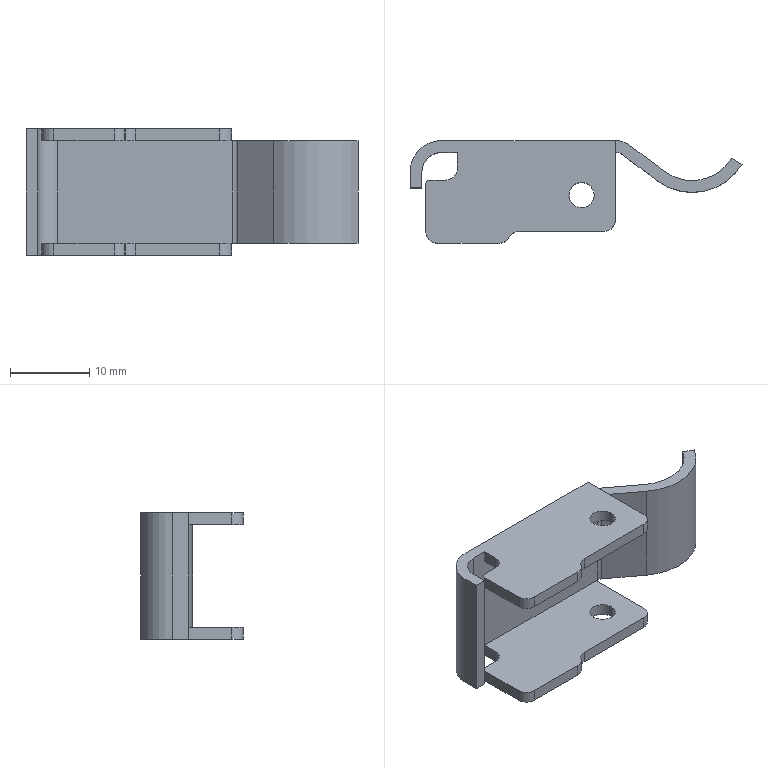Part | SolidWorks | features BaseBody 1 | 1 solid | 50 faces | box 42 x 13 x 16 mm | volume 1749 mm3 | plane 28 | cylinder 22 | commonest cylinder face diameters 3 x10 3.2 x4 1 x2 2 x1 5 x1 6 x1
STEP:
#1=CARTESIAN_POINT('',(36.4,3.,-8.));
#2=VERTEX_POINT('',#1);
#3=CARTESIAN_POINT('',(33.2,3.,-8.));
#4=VERTEX_POINT('',#3);
#5=CARTESIAN_POINT('',(34.8,3.,-8.));
#6=DIRECTION('',(0.,0.,-1.));
#7=DIRECTION('',(1.,0.,0.));
#8=AXIS2_PLACEMENT_3D('',#5,#6,#7);
#9=CIRCLE('',#8,1.6);
#10=EDGE_CURVE('',#2,#4,#9,.T.);
#11=ORIENTED_EDGE('',*,*,#10,.T.);
#12=CARTESIAN_POINT('',(33.2,3.,-6.5));
#13=VERTEX_POINT('',#12);
#14=CARTESIAN_POINT('',(33.2,3.,20.));
#15=DIRECTION('',(0.,0.,1.));
#16=VECTOR('',#15,1000.);
#17=LINE('',#14,#16);
#18=EDGE_CURVE('',#4,#13,#17,.T.);
#19=ORIENTED_EDGE('',*,*,#18,.T.);
#20=CARTESIAN_POINT('',(36.4,3.,-6.5));
#21=VERTEX_POINT('',#20);
#22=CARTESIAN_POINT('',(34.8,3.,-6.5));
#23=DIRECTION('',(0.,0.,-1.));
#24=DIRECTION('',(1.,0.,0.));
#25=AXIS2_PLACEMENT_3D('',#22,#23,#24);
#26=CIRCLE('',#25,1.6);
#27=EDGE_CURVE('',#21,#13,#26,.T.);
#28=ORIENTED_EDGE('',*,*,#27,.F.);
#29=CARTESIAN_POINT('',(36.4,3.,20.));
#30=DIRECTION('',(0.,0.,1.));
#31=VECTOR('',#30,1000.);
#32=LINE('',#29,#31);
#33=EDGE_CURVE('',#2,#21,#32,.T.);
#34=ORIENTED_EDGE('',*,*,#33,.F.);
#35=EDGE_LOOP('',(#11,#19,#28,#34));
#36=FACE_OUTER_BOUND('',#35,.T.);
#37=CARTESIAN_POINT('',(34.8,3.,20.));
#38=DIRECTION('',(0.,0.,1.));
#39=DIRECTION('',(1.,0.,0.));
#40=AXIS2_PLACEMENT_3D('',#37,#38,#39);
#41=CYLINDRICAL_SURFACE('',#40,1.6);
#42=ADVANCED_FACE('',(#36),#41,.F.);
#43=CARTESIAN_POINT('',(33.2,3.,6.5));
#44=VERTEX_POINT('',#43);
#45=CARTESIAN_POINT('',(36.4,3.,6.5));
#46=VERTEX_POINT('',#45);
#47=CARTESIAN_POINT('',(34.8,3.,6.5));
#48=DIRECTION('',(0.,0.,1.));
#49=DIRECTION('',(1.,0.,0.));
#50=AXIS2_PLACEMENT_3D('',#47,#48,#49);
#51=CIRCLE('',#50,1.6);
#52=EDGE_CURVE('',#44,#46,#51,.T.);
#53=ORIENTED_EDGE('',*,*,#52,.F.);
#54=CARTESIAN_POINT('',(33.2,3.,8.));
#55=VERTEX_POINT('',#54);
#56=CARTESIAN_POINT('',(33.2,3.,20.));
#57=DIRECTION('',(0.,0.,1.));
#58=VECTOR('',#57,1000.);
#59=LINE('',#56,#58);
#60=EDGE_CURVE('',#44,#55,#59,.T.);
#61=ORIENTED_EDGE('',*,*,#60,.T.);
#62=CARTESIAN_POINT('',(36.4,3.,8.));
#63=VERTEX_POINT('',#62);
#64=CARTESIAN_POINT('',(34.8,3.,8.));
#65=DIRECTION('',(0.,0.,-1.));
#66=DIRECTION('',(1.,0.,0.));
#67=AXIS2_PLACEMENT_3D('',#64,#65,#66);
#68=CIRCLE('',#67,1.6);
#69=EDGE_CURVE('',#63,#55,#68,.T.);
#70=ORIENTED_EDGE('',*,*,#69,.F.);
#71=CARTESIAN_POINT('',(36.4,3.,20.));
#72=DIRECTION('',(0.,0.,1.));
#73=VECTOR('',#72,1000.);
#74=LINE('',#71,#73);
#75=EDGE_CURVE('',#46,#63,#74,.T.);
#76=ORIENTED_EDGE('',*,*,#75,.F.);
#77=EDGE_LOOP('',(#53,#61,#70,#76));
#78=FACE_OUTER_BOUND('',#77,.T.);
#79=CARTESIAN_POINT('',(34.8,3.,20.));
#80=DIRECTION('',(0.,0.,1.));
#81=DIRECTION('',(1.,0.,0.));
#82=AXIS2_PLACEMENT_3D('',#79,#80,#81);
#83=CYLINDRICAL_SURFACE('',#82,1.6);
#84=ADVANCED_FACE('',(#78),#83,.F.);
#85=CARTESIAN_POINT('',(53.813,7.671,-6.5));
#86=VERTEX_POINT('',#85);
#87=CARTESIAN_POINT('',(53.813,7.671,6.5));
#88=VERTEX_POINT('',#87);
#89=CARTESIAN_POINT('',(53.813,7.671,8.));
#90=DIRECTION('',(0.,0.,1.));
#91=VECTOR('',#90,1000.);
#92=LINE('',#89,#91);
#93=EDGE_CURVE('',#86,#88,#92,.T.);
#94=ORIENTED_EDGE('',*,*,#93,.T.);
#95=CARTESIAN_POINT('',(55.1,6.9,6.5));
#96=VERTEX_POINT('',#95);
#97=CARTESIAN_POINT('',(55.1,6.9,6.5));
#98=DIRECTION('',(-0.8578,0.5139,0.));
#99=VECTOR('',#98,1000.);
#100=LINE('',#97,#99);
#101=EDGE_CURVE('',#96,#88,#100,.T.);
#102=ORIENTED_EDGE('',*,*,#101,.F.);
#103=CARTESIAN_POINT('',(55.1,6.9,-6.5));
#104=VERTEX_POINT('',#103);
#105=CARTESIAN_POINT('',(55.1,6.9,8.));
#106=DIRECTION('',(0.,0.,1.));
#107=VECTOR('',#106,1000.);
#108=LINE('',#105,#107);
#109=EDGE_CURVE('',#104,#96,#108,.T.);
#110=ORIENTED_EDGE('',*,*,#109,.F.);
#111=CARTESIAN_POINT('',(55.1,6.9,-6.5));
#112=DIRECTION('',(0.8578,-0.5139,0.));
#113=VECTOR('',#112,1000.);
#114=LINE('',#111,#113);
#115=EDGE_CURVE('',#86,#104,#114,.T.);
#116=ORIENTED_EDGE('',*,*,#115,.F.);
#117=EDGE_LOOP('',(#94,#102,#110,#116));
#118=FACE_OUTER_BOUND('',#117,.T.);
#119=CARTESIAN_POINT('',(55.1,6.9,8.));
#120=DIRECTION('',(-0.5139,-0.8578,0.));
#121=DIRECTION('',(-0.8578,0.5139,0.));
#122=AXIS2_PLACEMENT_3D('',#119,#120,#121);
#123=PLANE('',#122);
#124=ADVANCED_FACE('',(#118),#123,.F.);
#125=CARTESIAN_POINT('',(44.399,4.8,6.5));
#126=VERTEX_POINT('',#125);
#127=CARTESIAN_POINT('',(44.399,4.8,-6.5));
#128=VERTEX_POINT('',#127);
#129=CARTESIAN_POINT('',(44.399,4.8,8.));
#130=DIRECTION('',(0.,0.,-1.));
#131=VECTOR('',#130,1000.);
#132=LINE('',#129,#131);
#133=EDGE_CURVE('',#126,#128,#132,.T.);
#134=ORIENTED_EDGE('',*,*,#133,.F.);
#135=CARTESIAN_POINT('',(39.867,8.2,6.5));
#136=VERTEX_POINT('',#135);
#137=CARTESIAN_POINT('',(39.867,8.2,6.5));
#138=DIRECTION('',(0.8,-0.6,0.));
#139=VECTOR('',#138,1000.);
#140=LINE('',#137,#139);
#141=EDGE_CURVE('',#136,#126,#140,.T.);
#142=ORIENTED_EDGE('',*,*,#141,.F.);
#143=CARTESIAN_POINT('',(39.867,8.2,-6.5));
#144=VERTEX_POINT('',#143);
#145=CARTESIAN_POINT('',(39.867,8.2,8.));
#146=DIRECTION('',(0.,0.,-1.));
#147=VECTOR('',#146,1000.);
#148=LINE('',#145,#147);
#149=EDGE_CURVE('',#136,#144,#148,.T.);
#150=ORIENTED_EDGE('',*,*,#149,.T.);
#151=CARTESIAN_POINT('',(44.399,4.8,-6.5));
#152=DIRECTION('',(-0.8,0.6,0.));
#153=VECTOR('',#152,1000.);
#154=LINE('',#151,#153);
#155=EDGE_CURVE('',#128,#144,#154,.T.);
#156=ORIENTED_EDGE('',*,*,#155,.F.);
#157=EDGE_LOOP('',(#134,#142,#150,#156));
#158=FACE_OUTER_BOUND('',#157,.T.);
#159=CARTESIAN_POINT('',(39.867,8.2,8.));
#160=DIRECTION('',(0.6,0.8,0.));
#161=DIRECTION('',(0.,0.,-1.));
#162=AXIS2_PLACEMENT_3D('',#159,#160,#161);
#163=PLANE('',#162);
#164=ADVANCED_FACE('',(#158),#163,.F.);
#165=CARTESIAN_POINT('',(48.804,10.672,6.5));
#166=DIRECTION('',(0.,0.,1.));
#167=DIRECTION('',(1.,0.,0.));
#168=AXIS2_PLACEMENT_3D('',#165,#166,#167);
#169=CIRCLE('',#168,7.34);
#170=EDGE_CURVE('',#126,#96,#169,.T.);
#171=ORIENTED_EDGE('',*,*,#170,.F.);
#172=ORIENTED_EDGE('',*,*,#133,.T.);
#173=CARTESIAN_POINT('',(48.804,10.672,-6.5));
#174=DIRECTION('',(0.,0.,-1.));
#175=DIRECTION('',(1.,0.,0.));
#176=AXIS2_PLACEMENT_3D('',#173,#174,#175);
#177=CIRCLE('',#176,7.34);
#178=EDGE_CURVE('',#104,#128,#177,.T.);
#179=ORIENTED_EDGE('',*,*,#178,.F.);
#180=ORIENTED_EDGE('',*,*,#109,.T.);
#181=EDGE_LOOP('',(#171,#172,#179,#180));
#182=FACE_OUTER_BOUND('',#181,.T.);
#183=CARTESIAN_POINT('',(48.804,10.672,8.));
#184=DIRECTION('',(0.,0.,1.));
#185=DIRECTION('',(1.,0.,0.));
#186=AXIS2_PLACEMENT_3D('',#183,#184,#185);
#187=CYLINDRICAL_SURFACE('',#186,7.34);
#188=ADVANCED_FACE('',(#182),#187,.T.);
#189=CARTESIAN_POINT('',(45.299,6.,-6.5));
#190=VERTEX_POINT('',#189);
#191=CARTESIAN_POINT('',(48.803,10.672,-6.5));
#192=DIRECTION('',(0.,0.,1.));
#193=DIRECTION('',(1.,0.,0.));
#194=AXIS2_PLACEMENT_3D('',#191,#192,#193);
#195=CIRCLE('',#194,5.84);
#196=EDGE_CURVE('',#190,#86,#195,.T.);
#197=ORIENTED_EDGE('',*,*,#196,.F.);
#198=CARTESIAN_POINT('',(45.299,6.,6.5));
#199=VERTEX_POINT('',#198);
#200=CARTESIAN_POINT('',(45.299,6.,8.));
#201=DIRECTION('',(0.,0.,1.));
#202=VECTOR('',#201,1000.);
#203=LINE('',#200,#202);
#204=EDGE_CURVE('',#190,#199,#203,.T.);
#205=ORIENTED_EDGE('',*,*,#204,.T.);
#206=CARTESIAN_POINT('',(48.803,10.672,6.5));
#207=DIRECTION('',(0.,0.,-1.));
#208=DIRECTION('',(1.,0.,0.));
#209=AXIS2_PLACEMENT_3D('',#206,#207,#208);
#210=CIRCLE('',#209,5.84);
#211=EDGE_CURVE('',#88,#199,#210,.T.);
#212=ORIENTED_EDGE('',*,*,#211,.F.);
#213=ORIENTED_EDGE('',*,*,#93,.F.);
#214=EDGE_LOOP('',(#197,#205,#212,#213));
#215=FACE_OUTER_BOUND('',#214,.T.);
#216=CARTESIAN_POINT('',(48.803,10.672,8.));
#217=DIRECTION('',(0.,0.,1.));
#218=DIRECTION('',(1.,0.,0.));
#219=AXIS2_PLACEMENT_3D('',#216,#217,#218);
#220=CYLINDRICAL_SURFACE('',#219,5.84);
#221=ADVANCED_FACE('',(#215),#220,.F.);
#222=CARTESIAN_POINT('',(15.1,4.4,6.5));
#223=VERTEX_POINT('',#222);
#224=CARTESIAN_POINT('',(15.1,4.4,8.));
#225=VERTEX_POINT('',#224);
#226=CARTESIAN_POINT('',(15.1,4.4,8.));
#227=DIRECTION('',(0.,0.,1.));
#228=VECTOR('',#227,1000.);
#229=LINE('',#226,#228);
#230=EDGE_CURVE('',#223,#225,#229,.T.);
#231=ORIENTED_EDGE('',*,*,#230,.T.);
#232=CARTESIAN_POINT('',(15.6,4.9,8.));
#233=VERTEX_POINT('',#232);
#234=CARTESIAN_POINT('',(15.6,4.4,8.));
#235=DIRECTION('',(0.,0.,-1.));
#236=DIRECTION('',(1.,0.,0.));
#237=AXIS2_PLACEMENT_3D('',#234,#235,#236);
#238=CIRCLE('',#237,0.5);
#239=EDGE_CURVE('',#225,#233,#238,.T.);
#240=ORIENTED_EDGE('',*,*,#239,.T.);
#241=CARTESIAN_POINT('',(15.6,4.9,6.5));
#242=VERTEX_POINT('',#241);
#243=CARTESIAN_POINT('',(15.6,4.9,8.));
#244=DIRECTION('',(0.,0.,-1.));
#245=VECTOR('',#244,1000.);
#246=LINE('',#243,#245);
#247=EDGE_CURVE('',#233,#242,#246,.T.);
#248=ORIENTED_EDGE('',*,*,#247,.T.);
#249=CARTESIAN_POINT('',(15.6,4.4,6.5));
#250=DIRECTION('',(0.,0.,1.));
#251=DIRECTION('',(1.,0.,0.));
#252=AXIS2_PLACEMENT_3D('',#249,#250,#251);
#253=CIRCLE('',#252,0.5);
#254=EDGE_CURVE('',#242,#223,#253,.T.);
#255=ORIENTED_EDGE('',*,*,#254,.T.);
#256=EDGE_LOOP('',(#231,#240,#248,#255));
#257=FACE_OUTER_BOUND('',#256,.T.);
#258=CARTESIAN_POINT('',(15.6,4.4,8.));
#259=DIRECTION('',(0.,0.,1.));
#260=DIRECTION('',(1.,0.,0.));
#261=AXIS2_PLACEMENT_3D('',#258,#259,#260);
#262=CYLINDRICAL_SURFACE('',#261,0.5);
#263=ADVANCED_FACE('',(#257),#262,.T.);
#264=CARTESIAN_POINT('',(25.545,-2.432,6.5));
#265=VERTEX_POINT('',#264);
#266=CARTESIAN_POINT('',(25.655,-2.268,6.5));
#267=VERTEX_POINT('',#266);
#268=CARTESIAN_POINT('',(25.545,-2.432,6.5));
#269=DIRECTION('',(0.557,0.8305,0.));
#270=VECTOR('',#269,1000.);
#271=LINE('',#268,#270);
#272=EDGE_CURVE('',#265,#267,#271,.T.);
#273=ORIENTED_EDGE('',*,*,#272,.T.);
#274=CARTESIAN_POINT('',(25.655,-2.268,8.));
#275=VERTEX_POINT('',#274);
#276=CARTESIAN_POINT('',(25.655,-2.268,8.));
#277=DIRECTION('',(0.,0.,1.));
#278=VECTOR('',#277,1000.);
#279=LINE('',#276,#278);
#280=EDGE_CURVE('',#267,#275,#279,.T.);
#281=ORIENTED_EDGE('',*,*,#280,.T.);
#282=CARTESIAN_POINT('',(25.545,-2.432,8.));
#283=VERTEX_POINT('',#282);
#284=CARTESIAN_POINT('',(25.545,-2.432,8.));
#285=DIRECTION('',(0.557,0.8305,0.));
#286=VECTOR('',#285,1000.);
#287=LINE('',#284,#286);
#288=EDGE_CURVE('',#283,#275,#287,.T.);
#289=ORIENTED_EDGE('',*,*,#288,.F.);
#290=CARTESIAN_POINT('',(25.545,-2.432,8.));
#291=DIRECTION('',(0.,0.,1.));
#292=VECTOR('',#291,1000.);
#293=LINE('',#290,#292);
#294=EDGE_CURVE('',#265,#283,#293,.T.);
#295=ORIENTED_EDGE('',*,*,#294,.F.);
#296=EDGE_LOOP('',(#273,#281,#289,#295));
#297=FACE_OUTER_BOUND('',#296,.T.);
#298=CARTESIAN_POINT('',(25.545,-2.432,8.));
#299=DIRECTION('',(-0.8305,0.557,0.));
#300=DIRECTION('',(0.,0.,1.));
#301=AXIS2_PLACEMENT_3D('',#298,#299,#300);
#302=PLANE('',#301);
#303=ADVANCED_FACE('',(#297),#302,.F.);
#304=CARTESIAN_POINT('',(14.6,3.9,-8.));
#305=VERTEX_POINT('',#304);
#306=CARTESIAN_POINT('',(14.6,3.9,8.));
#307=VERTEX_POINT('',#306);
#308=CARTESIAN_POINT('',(14.6,3.9,8.));
#309=DIRECTION('',(0.,0.,1.));
#310=VECTOR('',#309,1000.);
#311=LINE('',#308,#310);
#312=EDGE_CURVE('',#305,#307,#311,.T.);
#313=ORIENTED_EDGE('',*,*,#312,.T.);
#314=CARTESIAN_POINT('',(13.1,3.9,8.));
#315=VERTEX_POINT('',#314);
#316=CARTESIAN_POINT('',(13.1,3.9,8.));
#317=DIRECTION('',(1.,0.,0.));
#318=VECTOR('',#317,1000.);
#319=LINE('',#316,#318);
#320=EDGE_CURVE('',#315,#307,#319,.T.);
#321=ORIENTED_EDGE('',*,*,#320,.F.);
#322=CARTESIAN_POINT('',(13.1,3.9,-8.));
#323=VERTEX_POINT('',#322);
#324=CARTESIAN_POINT('',(13.1,3.9,8.));
#325=DIRECTION('',(0.,0.,-1.));
#326=VECTOR('',#325,1000.);
#327=LINE('',#324,#326);
#328=EDGE_CURVE('',#315,#323,#327,.T.);
#329=ORIENTED_EDGE('',*,*,#328,.T.);
#330=CARTESIAN_POINT('',(13.1,3.9,-8.));
#331=DIRECTION('',(-1.,0.,0.));
#332=VECTOR('',#331,1000.);
#333=LINE('',#330,#332);
#334=EDGE_CURVE('',#305,#323,#333,.T.);
#335=ORIENTED_EDGE('',*,*,#334,.F.);
#336=EDGE_LOOP('',(#313,#321,#329,#335));
#337=FACE_OUTER_BOUND('',#336,.T.);
#338=CARTESIAN_POINT('',(13.1,3.9,8.));
#339=DIRECTION('',(0.,1.,0.));
#340=DIRECTION('',(1.,0.,0.));
#341=AXIS2_PLACEMENT_3D('',#338,#339,#340);
#342=PLANE('',#341);
#343=ADVANCED_FACE('',(#337),#342,.F.);
#344=CARTESIAN_POINT('',(34.8,3.,6.5));
#345=DIRECTION('',(0.,0.,1.));
#346=DIRECTION('',(1.,0.,0.));
#347=AXIS2_PLACEMENT_3D('',#344,#345,#346);
#348=CIRCLE('',#347,1.6);
#349=EDGE_CURVE('',#46,#44,#348,.T.);
#350=ORIENTED_EDGE('',*,*,#349,.T.);
#351=ORIENTED_EDGE('',*,*,#52,.T.);
#352=EDGE_LOOP('',(#350,#351));
#353=FACE_BOUND('',#352,.T.);
#354=CARTESIAN_POINT('',(39.1,8.4,6.5));
#355=VERTEX_POINT('',#354);
#356=CARTESIAN_POINT('',(39.1,-0.1,6.5));
#357=VERTEX_POINT('',#356);
#358=CARTESIAN_POINT('',(39.1,-0.1,6.5));
#359=DIRECTION('',(0.,-1.,0.));
#360=VECTOR('',#359,1000.);
#361=LINE('',#358,#360);
#362=EDGE_CURVE('',#355,#357,#361,.T.);
#363=ORIENTED_EDGE('',*,*,#362,.T.);
#364=CARTESIAN_POINT('',(37.6,-1.6,6.5));
#365=VERTEX_POINT('',#364);
#366=CARTESIAN_POINT('',(37.6,-0.1,6.5));
#367=DIRECTION('',(0.,0.,1.));
#368=DIRECTION('',(1.,0.,0.));
#369=AXIS2_PLACEMENT_3D('',#366,#367,#368);
#370=CIRCLE('',#369,1.5);
#371=EDGE_CURVE('',#365,#357,#370,.T.);
#372=ORIENTED_EDGE('',*,*,#371,.F.);
#373=CARTESIAN_POINT('',(26.903,-1.6,6.5));
#374=VERTEX_POINT('',#373);
#375=CARTESIAN_POINT('',(26.903,-1.6,6.5));
#376=DIRECTION('',(-1.,0.,0.));
#377=VECTOR('',#376,1000.);
#378=LINE('',#375,#377);
#379=EDGE_CURVE('',#365,#374,#378,.T.);
#380=ORIENTED_EDGE('',*,*,#379,.T.);
#381=CARTESIAN_POINT('',(26.903,-3.1,6.5));
#382=DIRECTION('',(0.,0.,1.));
#383=DIRECTION('',(1.,0.,0.));
#384=AXIS2_PLACEMENT_3D('',#381,#382,#383);
#385=CIRCLE('',#384,1.5);
#386=EDGE_CURVE('',#374,#267,#385,.T.);
#387=ORIENTED_EDGE('',*,*,#386,.T.);
#388=ORIENTED_EDGE('',*,*,#272,.F.);
#389=CARTESIAN_POINT('',(24.297,-3.1,6.5));
#390=VERTEX_POINT('',#389);
#391=CARTESIAN_POINT('',(24.297,-1.6,6.5));
#392=DIRECTION('',(0.,0.,1.));
#393=DIRECTION('',(1.,0.,0.));
#394=AXIS2_PLACEMENT_3D('',#391,#392,#393);
#395=CIRCLE('',#394,1.5);
#396=EDGE_CURVE('',#390,#265,#395,.T.);
#397=ORIENTED_EDGE('',*,*,#396,.F.);
#398=CARTESIAN_POINT('',(16.6,-3.1,6.5));
#399=VERTEX_POINT('',#398);
#400=CARTESIAN_POINT('',(16.6,-3.1,6.5));
#401=DIRECTION('',(-1.,0.,0.));
#402=VECTOR('',#401,1000.);
#403=LINE('',#400,#402);
#404=EDGE_CURVE('',#390,#399,#403,.T.);
#405=ORIENTED_EDGE('',*,*,#404,.T.);
#406=CARTESIAN_POINT('',(15.1,-1.6,6.5));
#407=VERTEX_POINT('',#406);
#408=CARTESIAN_POINT('',(16.6,-1.6,6.5));
#409=DIRECTION('',(0.,0.,1.));
#410=DIRECTION('',(1.,0.,0.));
#411=AXIS2_PLACEMENT_3D('',#408,#409,#410);
#412=CIRCLE('',#411,1.5);
#413=EDGE_CURVE('',#407,#399,#412,.T.);
#414=ORIENTED_EDGE('',*,*,#413,.F.);
#415=CARTESIAN_POINT('',(15.1,4.4,6.5));
#416=DIRECTION('',(0.,1.,0.));
#417=VECTOR('',#416,1000.);
#418=LINE('',#415,#417);
#419=EDGE_CURVE('',#407,#223,#418,.T.);
#420=ORIENTED_EDGE('',*,*,#419,.T.);
#421=ORIENTED_EDGE('',*,*,#254,.F.);
#422=CARTESIAN_POINT('',(17.6,4.9,6.5));
#423=VERTEX_POINT('',#422);
#424=CARTESIAN_POINT('',(17.6,4.9,6.5));
#425=DIRECTION('',(1.,0.,0.));
#426=VECTOR('',#425,1000.);
#427=LINE('',#424,#426);
#428=EDGE_CURVE('',#242,#423,#427,.T.);
#429=ORIENTED_EDGE('',*,*,#428,.T.);
#430=CARTESIAN_POINT('',(19.1,6.4,6.5));
#431=VERTEX_POINT('',#430);
#432=CARTESIAN_POINT('',(17.6,6.4,6.5));
#433=DIRECTION('',(0.,0.,1.));
#434=DIRECTION('',(1.,0.,0.));
#435=AXIS2_PLACEMENT_3D('',#432,#433,#434);
#436=CIRCLE('',#435,1.5);
#437=EDGE_CURVE('',#423,#431,#436,.T.);
#438=ORIENTED_EDGE('',*,*,#437,.T.);
#439=CARTESIAN_POINT('',(19.1,8.4,6.5));
#440=VERTEX_POINT('',#439);
#441=CARTESIAN_POINT('',(19.1,8.4,6.5));
#442=DIRECTION('',(0.,1.,0.));
#443=VECTOR('',#442,1000.);
#444=LINE('',#441,#443);
#445=EDGE_CURVE('',#431,#440,#444,.T.);
#446=ORIENTED_EDGE('',*,*,#445,.T.);
#447=CARTESIAN_POINT('',(39.1,8.4,6.5));
#448=DIRECTION('',(1.,0.,0.));
#449=VECTOR('',#448,1000.);
#450=LINE('',#447,#449);
#451=EDGE_CURVE('',#440,#355,#450,.T.);
#452=ORIENTED_EDGE('',*,*,#451,.T.);
#453=EDGE_LOOP('',(#363,#372,#380,#387,#388,#397,#405,#414,#420,#421,#429,#438,#446,#452));
#454=FACE_OUTER_BOUND('',#453,.T.);
#455=CARTESIAN_POINT('',(17.1,5.9,6.5));
#456=DIRECTION('',(0.,0.,1.));
#457=DIRECTION('',(1.,0.,0.));
#458=AXIS2_PLACEMENT_3D('',#455,#456,#457);
#459=PLANE('',#458);
#460=ADVANCED_FACE('',(#353,#454),#459,.F.);
#461=CARTESIAN_POINT('',(39.267,8.4,-6.5));
#462=VERTEX_POINT('',#461);
#463=CARTESIAN_POINT('',(39.267,7.4,-6.5));
#464=DIRECTION('',(0.,0.,1.));
#465=DIRECTION('',(1.,0.,0.));
#466=AXIS2_PLACEMENT_3D('',#463,#464,#465);
#467=CIRCLE('',#466,1.);
#468=EDGE_CURVE('',#144,#462,#467,.T.);
#469=ORIENTED_EDGE('',*,*,#468,.F.);
#470=ORIENTED_EDGE('',*,*,#149,.F.);
#471=CARTESIAN_POINT('',(39.267,8.4,6.5));
#472=VERTEX_POINT('',#471);
#473=CARTESIAN_POINT('',(39.267,7.4,6.5));
#474=DIRECTION('',(0.,0.,-1.));
#475=DIRECTION('',(1.,0.,0.));
#476=AXIS2_PLACEMENT_3D('',#473,#474,#475);
#477=CIRCLE('',#476,1.);
#478=EDGE_CURVE('',#472,#136,#477,.T.);
#479=ORIENTED_EDGE('',*,*,#478,.F.);
#480=CARTESIAN_POINT('',(39.267,8.4,8.));
#481=DIRECTION('',(0.,0.,-1.));
#482=VECTOR('',#481,1000.);
#483=LINE('',#480,#482);
#484=EDGE_CURVE('',#472,#462,#483,.T.);
#485=ORIENTED_EDGE('',*,*,#484,.T.);
#486=EDGE_LOOP('',(#469,#470,#479,#485));
#487=FACE_OUTER_BOUND('',#486,.T.);
#488=CARTESIAN_POINT('',(39.267,7.4,8.));
#489=DIRECTION('',(0.,0.,1.));
#490=DIRECTION('',(1.,0.,0.));
#491=AXIS2_PLACEMENT_3D('',#488,#489,#490);
#492=CYLINDRICAL_SURFACE('',#491,1.);
#493=ADVANCED_FACE('',(#487),#492,.F.);
#494=CARTESIAN_POINT('',(15.6,4.9,-8.));
#495=VERTEX_POINT('',#494);
#496=CARTESIAN_POINT('',(15.1,4.4,-8.));
#497=VERTEX_POINT('',#496);
#498=CARTESIAN_POINT('',(15.6,4.4,-8.));
#499=DIRECTION('',(0.,0.,1.));
#500=DIRECTION('',(1.,0.,0.));
#501=AXIS2_PLACEMENT_3D('',#498,#499,#500);
#502=CIRCLE('',#501,0.5);
#503=EDGE_CURVE('',#495,#497,#502,.T.);
#504=ORIENTED_EDGE('',*,*,#503,.T.);
#505=CARTESIAN_POINT('',(15.1,4.4,-6.5));
#506=VERTEX_POINT('',#505);
#507=CARTESIAN_POINT('',(15.1,4.4,8.));
#508=DIRECTION('',(0.,0.,1.));
#509=VECTOR('',#508,1000.);
#510=LINE('',#507,#509);
#511=EDGE_CURVE('',#497,#506,#510,.T.);
#512=ORIENTED_EDGE('',*,*,#511,.T.);
#513=CARTESIAN_POINT('',(15.6,4.9,-6.5));
#514=VERTEX_POINT('',#513);
#515=CARTESIAN_POINT('',(15.6,4.4,-6.5));
#516=DIRECTION('',(0.,0.,1.));
#517=DIRECTION('',(1.,0.,0.));
#518=AXIS2_PLACEMENT_3D('',#515,#516,#517);
#519=CIRCLE('',#518,0.5);
#520=EDGE_CURVE('',#514,#506,#519,.T.);
#521=ORIENTED_EDGE('',*,*,#520,.F.);
#522=CARTESIAN_POINT('',(15.6,4.9,8.));
#523=DIRECTION('',(0.,0.,-1.));
#524=VECTOR('',#523,1000.);
#525=LINE('',#522,#524);
#526=EDGE_CURVE('',#514,#495,#525,.T.);
#527=ORIENTED_EDGE('',*,*,#526,.T.);
#528=EDGE_LOOP('',(#504,#512,#521,#527));
#529=FACE_OUTER_BOUND('',#528,.T.);
#530=CARTESIAN_POINT('',(15.6,4.4,8.));
#531=DIRECTION('',(0.,0.,1.));
#532=DIRECTION('',(1.,0.,0.));
#533=AXIS2_PLACEMENT_3D('',#530,#531,#532);
#534=CYLINDRICAL_SURFACE('',#533,0.5);
#535=ADVANCED_FACE('',(#529),#534,.T.);
#536=CARTESIAN_POINT('',(25.545,-2.432,-8.));
#537=VERTEX_POINT('',#536);
#538=CARTESIAN_POINT('',(25.545,-2.432,-6.5));
#539=VERTEX_POINT('',#538);
#540=CARTESIAN_POINT('',(25.545,-2.432,8.));
#541=DIRECTION('',(0.,0.,1.));
#542=VECTOR('',#541,1000.);
#543=LINE('',#540,#542);
#544=EDGE_CURVE('',#537,#539,#543,.T.);
#545=ORIENTED_EDGE('',*,*,#544,.F.);
#546=CARTESIAN_POINT('',(25.655,-2.268,-8.));
#547=VERTEX_POINT('',#546);
#548=CARTESIAN_POINT('',(25.545,-2.432,-8.));
#549=DIRECTION('',(-0.557,-0.8305,0.));
#550=VECTOR('',#549,1000.);
#551=LINE('',#548,#550);
#552=EDGE_CURVE('',#547,#537,#551,.T.);
#553=ORIENTED_EDGE('',*,*,#552,.F.);
#554=CARTESIAN_POINT('',(25.655,-2.268,-6.5));
#555=VERTEX_POINT('',#554);
#556=CARTESIAN_POINT('',(25.655,-2.268,8.));
#557=DIRECTION('',(0.,0.,1.));
#558=VECTOR('',#557,1000.);
#559=LINE('',#556,#558);
#560=EDGE_CURVE('',#547,#555,#559,.T.);
#561=ORIENTED_EDGE('',*,*,#560,.T.);
#562=CARTESIAN_POINT('',(25.545,-2.432,-6.5));
#563=DIRECTION('',(0.557,0.8305,0.));
#564=VECTOR('',#563,1000.);
#565=LINE('',#562,#564);
#566=EDGE_CURVE('',#539,#555,#565,.T.);
#567=ORIENTED_EDGE('',*,*,#566,.F.);
#568=EDGE_LOOP('',(#545,#553,#561,#567));
#569=FACE_OUTER_BOUND('',#568,.T.);
#570=CARTESIAN_POINT('',(25.545,-2.432,8.));
#571=DIRECTION('',(-0.8305,0.557,0.));
#572=DIRECTION('',(0.,0.,1.));
#573=AXIS2_PLACEMENT_3D('',#570,#571,#572);
#574=PLANE('',#573);
#575=ADVANCED_FACE('',(#569),#574,.F.);
#576=ORIENTED_EDGE('',*,*,#27,.T.);
#577=CARTESIAN_POINT('',(34.8,3.,-6.5));
#578=DIRECTION('',(0.,0.,-1.));
#579=DIRECTION('',(1.,0.,0.));
#580=AXIS2_PLACEMENT_3D('',#577,#578,#579);
#581=CIRCLE('',#580,1.6);
#582=EDGE_CURVE('',#13,#21,#581,.T.);
#583=ORIENTED_EDGE('',*,*,#582,.T.);
#584=EDGE_LOOP('',(#576,#583));
#585=FACE_BOUND('',#584,.T.);
#586=CARTESIAN_POINT('',(39.1,-0.1,-6.5));
#587=VERTEX_POINT('',#586);
#588=CARTESIAN_POINT('',(39.1,8.4,-6.5));
#589=VERTEX_POINT('',#588);
#590=CARTESIAN_POINT('',(39.1,-0.1,-6.5));
#591=DIRECTION('',(0.,1.,0.));
#592=VECTOR('',#591,1000.);
#593=LINE('',#590,#592);
#594=EDGE_CURVE('',#587,#589,#593,.T.);
#595=ORIENTED_EDGE('',*,*,#594,.T.);
#596=CARTESIAN_POINT('',(19.1,8.4,-6.5));
#597=VERTEX_POINT('',#596);
#598=CARTESIAN_POINT('',(39.1,8.4,-6.5));
#599=DIRECTION('',(-1.,0.,0.));
#600=VECTOR('',#599,1000.);
#601=LINE('',#598,#600);
#602=EDGE_CURVE('',#589,#597,#601,.T.);
#603=ORIENTED_EDGE('',*,*,#602,.T.);
#604=CARTESIAN_POINT('',(19.1,6.4,-6.5));
#605=VERTEX_POINT('',#604);
#606=CARTESIAN_POINT('',(19.1,8.4,-6.5));
#607=DIRECTION('',(0.,-1.,0.));
#608=VECTOR('',#607,1000.);
#609=LINE('',#606,#608);
#610=EDGE_CURVE('',#597,#605,#609,.T.);
#611=ORIENTED_EDGE('',*,*,#610,.T.);
#612=CARTESIAN_POINT('',(17.6,4.9,-6.5));
#613=VERTEX_POINT('',#612);
#614=CARTESIAN_POINT('',(17.6,6.4,-6.5));
#615=DIRECTION('',(0.,0.,-1.));
#616=DIRECTION('',(1.,0.,0.));
#617=AXIS2_PLACEMENT_3D('',#614,#615,#616);
#618=CIRCLE('',#617,1.5);
#619=EDGE_CURVE('',#605,#613,#618,.T.);
#620=ORIENTED_EDGE('',*,*,#619,.T.);
#621=CARTESIAN_POINT('',(17.6,4.9,-6.5));
#622=DIRECTION('',(-1.,0.,0.));
#623=VECTOR('',#622,1000.);
#624=LINE('',#621,#623);
#625=EDGE_CURVE('',#613,#514,#624,.T.);
#626=ORIENTED_EDGE('',*,*,#625,.T.);
#627=ORIENTED_EDGE('',*,*,#520,.T.);
#628=CARTESIAN_POINT('',(15.1,-1.6,-6.5));
#629=VERTEX_POINT('',#628);
#630=CARTESIAN_POINT('',(15.1,4.4,-6.5));
#631=DIRECTION('',(0.,-1.,0.));
#632=VECTOR('',#631,1000.);
#633=LINE('',#630,#632);
#634=EDGE_CURVE('',#506,#629,#633,.T.);
#635=ORIENTED_EDGE('',*,*,#634,.T.);
#636=CARTESIAN_POINT('',(16.6,-3.1,-6.5));
#637=VERTEX_POINT('',#636);
#638=CARTESIAN_POINT('',(16.6,-1.6,-6.5));
#639=DIRECTION('',(0.,0.,-1.));
#640=DIRECTION('',(1.,0.,0.));
#641=AXIS2_PLACEMENT_3D('',#638,#639,#640);
#642=CIRCLE('',#641,1.5);
#643=EDGE_CURVE('',#637,#629,#642,.T.);
#644=ORIENTED_EDGE('',*,*,#643,.F.);
#645=CARTESIAN_POINT('',(24.297,-3.1,-6.5));
#646=VERTEX_POINT('',#645);
#647=CARTESIAN_POINT('',(16.6,-3.1,-6.5));
#648=DIRECTION('',(1.,0.,0.));
#649=VECTOR('',#648,1000.);
#650=LINE('',#647,#649);
#651=EDGE_CURVE('',#637,#646,#650,.T.);
#652=ORIENTED_EDGE('',*,*,#651,.T.);
#653=CARTESIAN_POINT('',(24.297,-1.6,-6.5));
#654=DIRECTION('',(0.,0.,-1.));
#655=DIRECTION('',(1.,0.,0.));
#656=AXIS2_PLACEMENT_3D('',#653,#654,#655);
#657=CIRCLE('',#656,1.5);
#658=EDGE_CURVE('',#539,#646,#657,.T.);
#659=ORIENTED_EDGE('',*,*,#658,.F.);
#660=ORIENTED_EDGE('',*,*,#566,.T.);
#661=CARTESIAN_POINT('',(26.903,-1.6,-6.5));
#662=VERTEX_POINT('',#661);
#663=CARTESIAN_POINT('',(26.903,-3.1,-6.5));
#664=DIRECTION('',(0.,0.,-1.));
#665=DIRECTION('',(1.,0.,0.));
#666=AXIS2_PLACEMENT_3D('',#663,#664,#665);
#667=CIRCLE('',#666,1.5);
#668=EDGE_CURVE('',#555,#662,#667,.T.);
#669=ORIENTED_EDGE('',*,*,#668,.T.);
#670=CARTESIAN_POINT('',(37.6,-1.6,-6.5));
#671=VERTEX_POINT('',#670);
#672=CARTESIAN_POINT('',(26.903,-1.6,-6.5));
#673=DIRECTION('',(1.,0.,0.));
#674=VECTOR('',#673,1000.);
#675=LINE('',#672,#674);
#676=EDGE_CURVE('',#662,#671,#675,.T.);
#677=ORIENTED_EDGE('',*,*,#676,.T.);
#678=CARTESIAN_POINT('',(37.6,-0.1,-6.5));
#679=DIRECTION('',(0.,0.,-1.));
#680=DIRECTION('',(1.,0.,0.));
#681=AXIS2_PLACEMENT_3D('',#678,#679,#680);
#682=CIRCLE('',#681,1.5);
#683=EDGE_CURVE('',#587,#671,#682,.T.);
#684=ORIENTED_EDGE('',*,*,#683,.F.);
#685=EDGE_LOOP('',(#595,#603,#611,#620,#626,#627,#635,#644,#652,#659,#660,#669,#677,#684));
#686=FACE_OUTER_BOUND('',#685,.T.);
#687=CARTESIAN_POINT('',(17.1,5.9,-6.5));
#688=DIRECTION('',(0.,0.,1.));
#689=DIRECTION('',(1.,0.,0.));
#690=AXIS2_PLACEMENT_3D('',#687,#688,#689);
#691=PLANE('',#690);
#692=ADVANCED_FACE('',(#585,#686),#691,.T.);
#693=ORIENTED_EDGE('',*,*,#155,.T.);
#694=ORIENTED_EDGE('',*,*,#468,.T.);
#695=CARTESIAN_POINT('',(39.1,8.4,-6.5));
#696=DIRECTION('',(-1.,0.,0.));
#697=VECTOR('',#696,1000.);
#698=LINE('',#695,#697);
#699=EDGE_CURVE('',#462,#589,#698,.T.);
#700=ORIENTED_EDGE('',*,*,#699,.T.);
#701=CARTESIAN_POINT('',(39.1,9.9,-6.5));
#702=VERTEX_POINT('',#701);
#703=CARTESIAN_POINT('',(39.1,-0.1,-6.5));
#704=DIRECTION('',(0.,1.,0.));
#705=VECTOR('',#704,1000.);
#706=LINE('',#703,#705);
#707=EDGE_CURVE('',#589,#702,#706,.T.);
#708=ORIENTED_EDGE('',*,*,#707,.T.);
#709=CARTESIAN_POINT('',(40.9,9.3,-6.5));
#710=VERTEX_POINT('',#709);
#711=CARTESIAN_POINT('',(39.1,6.9,-6.5));
#712=DIRECTION('',(0.,0.,1.));
#713=DIRECTION('',(1.,0.,0.));
#714=AXIS2_PLACEMENT_3D('',#711,#712,#713);
#715=CIRCLE('',#714,3.);
#716=EDGE_CURVE('',#710,#702,#715,.T.);
#717=ORIENTED_EDGE('',*,*,#716,.F.);
#718=CARTESIAN_POINT('',(45.299,6.,-6.5));
#719=DIRECTION('',(0.8,-0.6,0.));
#720=VECTOR('',#719,1000.);
#721=LINE('',#718,#720);
#722=EDGE_CURVE('',#710,#190,#721,.T.);
#723=ORIENTED_EDGE('',*,*,#722,.T.);
#724=ORIENTED_EDGE('',*,*,#196,.T.);
#725=ORIENTED_EDGE('',*,*,#115,.T.);
#726=ORIENTED_EDGE('',*,*,#178,.T.);
#727=EDGE_LOOP('',(#693,#694,#700,#708,#717,#723,#724,#725,#726));
#728=FACE_OUTER_BOUND('',#727,.T.);
#729=CARTESIAN_POINT('',(39.1,20.,-6.5));
#730=DIRECTION('',(0.,0.,-1.));
#731=DIRECTION('',(0.,-1.,0.));
#732=AXIS2_PLACEMENT_3D('',#729,#730,#731);
#733=PLANE('',#732);
#734=ADVANCED_FACE('',(#728),#733,.T.);
#735=CARTESIAN_POINT('',(39.1,9.9,6.5));
#736=VERTEX_POINT('',#735);
#737=CARTESIAN_POINT('',(40.9,9.3,6.5));
#738=VERTEX_POINT('',#737);
#739=CARTESIAN_POINT('',(39.1,6.9,6.5));
#740=DIRECTION('',(0.,0.,-1.));
#741=DIRECTION('',(1.,0.,0.));
#742=AXIS2_PLACEMENT_3D('',#739,#740,#741);
#743=CIRCLE('',#742,3.);
#744=EDGE_CURVE('',#736,#738,#743,.T.);
#745=ORIENTED_EDGE('',*,*,#744,.F.);
#746=CARTESIAN_POINT('',(39.1,-0.1,6.5));
#747=DIRECTION('',(0.,-1.,0.));
#748=VECTOR('',#747,1000.);
#749=LINE('',#746,#748);
#750=EDGE_CURVE('',#736,#355,#749,.T.);
#751=ORIENTED_EDGE('',*,*,#750,.T.);
#752=CARTESIAN_POINT('',(39.1,8.4,6.5));
#753=DIRECTION('',(1.,0.,0.));
#754=VECTOR('',#753,1000.);
#755=LINE('',#752,#754);
#756=EDGE_CURVE('',#355,#472,#755,.T.);
#757=ORIENTED_EDGE('',*,*,#756,.T.);
#758=ORIENTED_EDGE('',*,*,#478,.T.);
#759=ORIENTED_EDGE('',*,*,#141,.T.);
#760=ORIENTED_EDGE('',*,*,#170,.T.);
#761=ORIENTED_EDGE('',*,*,#101,.T.);
#762=ORIENTED_EDGE('',*,*,#211,.T.);
#763=CARTESIAN_POINT('',(45.299,6.,6.5));
#764=DIRECTION('',(-0.8,0.6,0.));
#765=VECTOR('',#764,1000.);
#766=LINE('',#763,#765);
#767=EDGE_CURVE('',#199,#738,#766,.T.);
#768=ORIENTED_EDGE('',*,*,#767,.T.);
#769=EDGE_LOOP('',(#745,#751,#757,#758,#759,#760,#761,#762,#768));
#770=FACE_OUTER_BOUND('',#769,.T.);
#771=CARTESIAN_POINT('',(56.1,20.,6.5));
#772=DIRECTION('',(0.,0.,1.));
#773=DIRECTION('',(1.,0.,0.));
#774=AXIS2_PLACEMENT_3D('',#771,#772,#773);
#775=PLANE('',#774);
#776=ADVANCED_FACE('',(#770),#775,.T.);
#777=CARTESIAN_POINT('',(40.9,9.3,8.));
#778=DIRECTION('',(0.,0.,-1.));
#779=VECTOR('',#778,1000.);
#780=LINE('',#777,#779);
#781=EDGE_CURVE('',#738,#710,#780,.T.);
#782=ORIENTED_EDGE('',*,*,#781,.F.);
#783=ORIENTED_EDGE('',*,*,#767,.F.);
#784=ORIENTED_EDGE('',*,*,#204,.F.);
#785=ORIENTED_EDGE('',*,*,#722,.F.);
#786=EDGE_LOOP('',(#782,#783,#784,#785));
#787=FACE_OUTER_BOUND('',#786,.T.);
#788=CARTESIAN_POINT('',(45.299,6.,8.));
#789=DIRECTION('',(-0.6,-0.8,0.));
#790=DIRECTION('',(-0.8,0.6,0.));
#791=AXIS2_PLACEMENT_3D('',#788,#789,#790);
#792=PLANE('',#791);
#793=ADVANCED_FACE('',(#787),#792,.F.);
#794=ORIENTED_EDGE('',*,*,#362,.F.);
#795=ORIENTED_EDGE('',*,*,#750,.F.);
#796=CARTESIAN_POINT('',(39.1,9.9,8.));
#797=VERTEX_POINT('',#796);
#798=CARTESIAN_POINT('',(39.1,9.9,8.));
#799=DIRECTION('',(0.,0.,-1.));
#800=VECTOR('',#799,1000.);
#801=LINE('',#798,#800);
#802=EDGE_CURVE('',#797,#736,#801,.T.);
#803=ORIENTED_EDGE('',*,*,#802,.F.);
#804=CARTESIAN_POINT('',(39.1,-0.1,8.));
#805=VERTEX_POINT('',#804);
#806=CARTESIAN_POINT('',(39.1,5.9,8.));
#807=DIRECTION('',(0.,1.,0.));
#808=VECTOR('',#807,1000.);
#809=LINE('',#806,#808);
#810=EDGE_CURVE('',#805,#797,#809,.T.);
#811=ORIENTED_EDGE('',*,*,#810,.F.);
#812=CARTESIAN_POINT('',(39.1,-0.1,8.));
#813=DIRECTION('',(0.,0.,1.));
#814=VECTOR('',#813,1000.);
#815=LINE('',#812,#814);
#816=EDGE_CURVE('',#357,#805,#815,.T.);
#817=ORIENTED_EDGE('',*,*,#816,.F.);
#818=EDGE_LOOP('',(#794,#795,#803,#811,#817));
#819=FACE_OUTER_BOUND('',#818,.T.);
#820=CARTESIAN_POINT('',(39.1,-0.1,8.));
#821=DIRECTION('',(-1.,0.,0.));
#822=DIRECTION('',(0.,0.,1.));
#823=AXIS2_PLACEMENT_3D('',#820,#821,#822);
#824=PLANE('',#823);
#825=ADVANCED_FACE('',(#819),#824,.F.);
#826=ORIENTED_EDGE('',*,*,#445,.F.);
#827=CARTESIAN_POINT('',(19.1,6.4,8.));
#828=VERTEX_POINT('',#827);
#829=CARTESIAN_POINT('',(19.1,6.4,8.));
#830=DIRECTION('',(0.,0.,1.));
#831=VECTOR('',#830,1000.);
#832=LINE('',#829,#831);
#833=EDGE_CURVE('',#431,#828,#832,.T.);
#834=ORIENTED_EDGE('',*,*,#833,.T.);
#835=CARTESIAN_POINT('',(19.1,8.4,8.));
#836=VERTEX_POINT('',#835);
#837=CARTESIAN_POINT('',(19.1,5.9,8.));
#838=DIRECTION('',(0.,-1.,0.));
#839=VECTOR('',#838,1000.);
#840=LINE('',#837,#839);
#841=EDGE_CURVE('',#836,#828,#840,.T.);
#842=ORIENTED_EDGE('',*,*,#841,.F.);
#843=CARTESIAN_POINT('',(19.1,8.4,8.));
#844=DIRECTION('',(0.,0.,-1.));
#845=VECTOR('',#844,1000.);
#846=LINE('',#843,#845);
#847=EDGE_CURVE('',#836,#440,#846,.T.);
#848=ORIENTED_EDGE('',*,*,#847,.T.);
#849=EDGE_LOOP('',(#826,#834,#842,#848));
#850=FACE_OUTER_BOUND('',#849,.T.);
#851=CARTESIAN_POINT('',(19.1,8.4,8.));
#852=DIRECTION('',(1.,0.,0.));
#853=DIRECTION('',(0.,1.,0.));
#854=AXIS2_PLACEMENT_3D('',#851,#852,#853);
#855=PLANE('',#854);
#856=ADVANCED_FACE('',(#850),#855,.F.);
#857=CARTESIAN_POINT('',(17.6,4.9,8.));
#858=VERTEX_POINT('',#857);
#859=CARTESIAN_POINT('',(17.6,4.9,8.));
#860=DIRECTION('',(0.,0.,1.));
#861=VECTOR('',#860,1000.);
#862=LINE('',#859,#861);
#863=EDGE_CURVE('',#423,#858,#862,.T.);
#864=ORIENTED_EDGE('',*,*,#863,.T.);
#865=CARTESIAN_POINT('',(17.6,6.4,8.));
#866=DIRECTION('',(0.,0.,-1.));
#867=DIRECTION('',(1.,0.,0.));
#868=AXIS2_PLACEMENT_3D('',#865,#866,#867);
#869=CIRCLE('',#868,1.5);
#870=EDGE_CURVE('',#828,#858,#869,.T.);
#871=ORIENTED_EDGE('',*,*,#870,.F.);
#872=ORIENTED_EDGE('',*,*,#833,.F.);
#873=ORIENTED_EDGE('',*,*,#437,.F.);
#874=EDGE_LOOP('',(#864,#871,#872,#873));
#875=FACE_OUTER_BOUND('',#874,.T.);
#876=CARTESIAN_POINT('',(17.6,6.4,8.));
#877=DIRECTION('',(0.,0.,1.));
#878=DIRECTION('',(1.,0.,0.));
#879=AXIS2_PLACEMENT_3D('',#876,#877,#878);
#880=CYLINDRICAL_SURFACE('',#879,1.5);
#881=ADVANCED_FACE('',(#875),#880,.F.);
#882=ORIENTED_EDGE('',*,*,#428,.F.);
#883=ORIENTED_EDGE('',*,*,#247,.F.);
#884=CARTESIAN_POINT('',(17.1,4.9,8.));
#885=DIRECTION('',(-1.,0.,0.));
#886=VECTOR('',#885,1000.);
#887=LINE('',#884,#886);
#888=EDGE_CURVE('',#858,#233,#887,.T.);
#889=ORIENTED_EDGE('',*,*,#888,.F.);
#890=ORIENTED_EDGE('',*,*,#863,.F.);
#891=EDGE_LOOP('',(#882,#883,#889,#890));
#892=FACE_OUTER_BOUND('',#891,.T.);
#893=CARTESIAN_POINT('',(17.6,4.9,8.));
#894=DIRECTION('',(0.,-1.,0.));
#895=DIRECTION('',(0.,0.,-1.));
#896=AXIS2_PLACEMENT_3D('',#893,#894,#895);
#897=PLANE('',#896);
#898=ADVANCED_FACE('',(#892),#897,.F.);
#899=ORIENTED_EDGE('',*,*,#419,.F.);
#900=CARTESIAN_POINT('',(15.1,-1.6,8.));
#901=VERTEX_POINT('',#900);
#902=CARTESIAN_POINT('',(15.1,-1.6,8.));
#903=DIRECTION('',(0.,0.,-1.));
#904=VECTOR('',#903,1000.);
#905=LINE('',#902,#904);
#906=EDGE_CURVE('',#901,#407,#905,.T.);
#907=ORIENTED_EDGE('',*,*,#906,.F.);
#908=CARTESIAN_POINT('',(15.1,5.9,8.));
#909=DIRECTION('',(0.,-1.,0.));
#910=VECTOR('',#909,1000.);
#911=LINE('',#908,#910);
#912=EDGE_CURVE('',#225,#901,#911,.T.);
#913=ORIENTED_EDGE('',*,*,#912,.F.);
#914=ORIENTED_EDGE('',*,*,#230,.F.);
#915=EDGE_LOOP('',(#899,#907,#913,#914));
#916=FACE_OUTER_BOUND('',#915,.T.);
#917=CARTESIAN_POINT('',(15.1,4.4,8.));
#918=DIRECTION('',(1.,0.,0.));
#919=DIRECTION('',(0.,1.,0.));
#920=AXIS2_PLACEMENT_3D('',#917,#918,#919);
#921=PLANE('',#920);
#922=ADVANCED_FACE('',(#916),#921,.F.);
#923=CARTESIAN_POINT('',(16.6,-3.1,8.));
#924=VERTEX_POINT('',#923);
#925=CARTESIAN_POINT('',(16.6,-3.1,8.));
#926=DIRECTION('',(0.,0.,1.));
#927=VECTOR('',#926,1000.);
#928=LINE('',#925,#927);
#929=EDGE_CURVE('',#399,#924,#928,.T.);
#930=ORIENTED_EDGE('',*,*,#929,.T.);
#931=CARTESIAN_POINT('',(16.6,-1.6,8.));
#932=DIRECTION('',(0.,0.,1.));
#933=DIRECTION('',(1.,0.,0.));
#934=AXIS2_PLACEMENT_3D('',#931,#932,#933);
#935=CIRCLE('',#934,1.5);
#936=EDGE_CURVE('',#901,#924,#935,.T.);
#937=ORIENTED_EDGE('',*,*,#936,.F.);
#938=ORIENTED_EDGE('',*,*,#906,.T.);
#939=ORIENTED_EDGE('',*,*,#413,.T.);
#940=EDGE_LOOP('',(#930,#937,#938,#939));
#941=FACE_OUTER_BOUND('',#940,.T.);
#942=CARTESIAN_POINT('',(16.6,-1.6,8.));
#943=DIRECTION('',(0.,0.,1.));
#944=DIRECTION('',(1.,0.,0.));
#945=AXIS2_PLACEMENT_3D('',#942,#943,#944);
#946=CYLINDRICAL_SURFACE('',#945,1.5);
#947=ADVANCED_FACE('',(#941),#946,.T.);
#948=ORIENTED_EDGE('',*,*,#404,.F.);
#949=CARTESIAN_POINT('',(24.297,-3.1,8.));
#950=VERTEX_POINT('',#949);
#951=CARTESIAN_POINT('',(24.297,-3.1,8.));
#952=DIRECTION('',(0.,0.,-1.));
#953=VECTOR('',#952,1000.);
#954=LINE('',#951,#953);
#955=EDGE_CURVE('',#950,#390,#954,.T.);
#956=ORIENTED_EDGE('',*,*,#955,.F.);
#957=CARTESIAN_POINT('',(17.1,-3.1,8.));
#958=DIRECTION('',(1.,0.,0.));
#959=VECTOR('',#958,1000.);
#960=LINE('',#957,#959);
#961=EDGE_CURVE('',#924,#950,#960,.T.);
#962=ORIENTED_EDGE('',*,*,#961,.F.);
#963=ORIENTED_EDGE('',*,*,#929,.F.);
#964=EDGE_LOOP('',(#948,#956,#962,#963));
#965=FACE_OUTER_BOUND('',#964,.T.);
#966=CARTESIAN_POINT('',(16.6,-3.1,8.));
#967=DIRECTION('',(0.,1.,0.));
#968=DIRECTION('',(1.,0.,0.));
#969=AXIS2_PLACEMENT_3D('',#966,#967,#968);
#970=PLANE('',#969);
#971=ADVANCED_FACE('',(#965),#970,.F.);
#972=ORIENTED_EDGE('',*,*,#294,.T.);
#973=CARTESIAN_POINT('',(24.297,-1.6,8.));
#974=DIRECTION('',(0.,0.,1.));
#975=DIRECTION('',(1.,0.,0.));
#976=AXIS2_PLACEMENT_3D('',#973,#974,#975);
#977=CIRCLE('',#976,1.5);
#978=EDGE_CURVE('',#950,#283,#977,.T.);
#979=ORIENTED_EDGE('',*,*,#978,.F.);
#980=ORIENTED_EDGE('',*,*,#955,.T.);
#981=ORIENTED_EDGE('',*,*,#396,.T.);
#982=EDGE_LOOP('',(#972,#979,#980,#981));
#983=FACE_OUTER_BOUND('',#982,.T.);
#984=CARTESIAN_POINT('',(24.297,-1.6,8.));
#985=DIRECTION('',(0.,0.,1.));
#986=DIRECTION('',(1.,0.,0.));
#987=AXIS2_PLACEMENT_3D('',#984,#985,#986);
#988=CYLINDRICAL_SURFACE('',#987,1.5);
#989=ADVANCED_FACE('',(#983),#988,.T.);
#990=CARTESIAN_POINT('',(26.903,-1.6,8.));
#991=VERTEX_POINT('',#990);
#992=CARTESIAN_POINT('',(26.903,-1.6,8.));
#993=DIRECTION('',(0.,0.,1.));
#994=VECTOR('',#993,1000.);
#995=LINE('',#992,#994);
#996=EDGE_CURVE('',#374,#991,#995,.T.);
#997=ORIENTED_EDGE('',*,*,#996,.T.);
#998=CARTESIAN_POINT('',(26.903,-3.1,8.));
#999=DIRECTION('',(0.,0.,-1.));
#1000=DIRECTION('',(1.,0.,0.));
#1001=AXIS2_PLACEMENT_3D('',#998,#999,#1000);
#1002=CIRCLE('',#1001,1.5);
#1003=EDGE_CURVE('',#275,#991,#1002,.T.);
#1004=ORIENTED_EDGE('',*,*,#1003,.F.);
#1005=ORIENTED_EDGE('',*,*,#280,.F.);
#1006=ORIENTED_EDGE('',*,*,#386,.F.);
#1007=EDGE_LOOP('',(#997,#1004,#1005,#1006));
#1008=FACE_OUTER_BOUND('',#1007,.T.);
#1009=CARTESIAN_POINT('',(26.903,-3.1,8.));
#1010=DIRECTION('',(0.,0.,1.));
#1011=DIRECTION('',(1.,0.,0.));
#1012=AXIS2_PLACEMENT_3D('',#1009,#1010,#1011);
#1013=CYLINDRICAL_SURFACE('',#1012,1.5);
#1014=ADVANCED_FACE('',(#1008),#1013,.F.);
#1015=ORIENTED_EDGE('',*,*,#379,.F.);
#1016=CARTESIAN_POINT('',(37.6,-1.6,8.));
#1017=VERTEX_POINT('',#1016);
#1018=CARTESIAN_POINT('',(37.6,-1.6,8.));
#1019=DIRECTION('',(0.,0.,-1.));
#1020=VECTOR('',#1019,1000.);
#1021=LINE('',#1018,#1020);
#1022=EDGE_CURVE('',#1017,#365,#1021,.T.);
#1023=ORIENTED_EDGE('',*,*,#1022,.F.);
#1024=CARTESIAN_POINT('',(17.1,-1.6,8.));
#1025=DIRECTION('',(1.,0.,0.));
#1026=VECTOR('',#1025,1000.);
#1027=LINE('',#1024,#1026);
#1028=EDGE_CURVE('',#991,#1017,#1027,.T.);
#1029=ORIENTED_EDGE('',*,*,#1028,.F.);
#1030=ORIENTED_EDGE('',*,*,#996,.F.);
#1031=EDGE_LOOP('',(#1015,#1023,#1029,#1030));
#1032=FACE_OUTER_BOUND('',#1031,.T.);
#1033=CARTESIAN_POINT('',(26.903,-1.6,8.));
#1034=DIRECTION('',(0.,1.,0.));
#1035=DIRECTION('',(1.,0.,0.));
#1036=AXIS2_PLACEMENT_3D('',#1033,#1034,#1035);
#1037=PLANE('',#1036);
#1038=ADVANCED_FACE('',(#1032),#1037,.F.);
#1039=ORIENTED_EDGE('',*,*,#816,.T.);
#1040=CARTESIAN_POINT('',(37.6,-0.1,8.));
#1041=DIRECTION('',(0.,0.,1.));
#1042=DIRECTION('',(1.,0.,0.));
#1043=AXIS2_PLACEMENT_3D('',#1040,#1041,#1042);
#1044=CIRCLE('',#1043,1.5);
#1045=EDGE_CURVE('',#1017,#805,#1044,.T.);
#1046=ORIENTED_EDGE('',*,*,#1045,.F.);
#1047=ORIENTED_EDGE('',*,*,#1022,.T.);
#1048=ORIENTED_EDGE('',*,*,#371,.T.);
#1049=EDGE_LOOP('',(#1039,#1046,#1047,#1048));
#1050=FACE_OUTER_BOUND('',#1049,.T.);
#1051=CARTESIAN_POINT('',(37.6,-0.1,8.));
#1052=DIRECTION('',(0.,0.,1.));
#1053=DIRECTION('',(1.,0.,0.));
#1054=AXIS2_PLACEMENT_3D('',#1051,#1052,#1053);
#1055=CYLINDRICAL_SURFACE('',#1054,1.5);
#1056=ADVANCED_FACE('',(#1050),#1055,.T.);
#1057=ORIENTED_EDGE('',*,*,#328,.F.);
#1058=CARTESIAN_POINT('',(13.1,5.9,8.));
#1059=VERTEX_POINT('',#1058);
#1060=CARTESIAN_POINT('',(13.1,5.9,8.));
#1061=DIRECTION('',(0.,-1.,0.));
#1062=VECTOR('',#1061,1000.);
#1063=LINE('',#1060,#1062);
#1064=EDGE_CURVE('',#1059,#315,#1063,.T.);
#1065=ORIENTED_EDGE('',*,*,#1064,.F.);
#1066=CARTESIAN_POINT('',(13.1,5.9,-8.));
#1067=VERTEX_POINT('',#1066);
#1068=CARTESIAN_POINT('',(13.1,5.9,8.));
#1069=DIRECTION('',(0.,0.,1.));
#1070=VECTOR('',#1069,1000.);
#1071=LINE('',#1068,#1070);
#1072=EDGE_CURVE('',#1067,#1059,#1071,.T.);
#1073=ORIENTED_EDGE('',*,*,#1072,.F.);
#1074=CARTESIAN_POINT('',(13.1,5.9,-8.));
#1075=DIRECTION('',(0.,-1.,0.));
#1076=VECTOR('',#1075,1000.);
#1077=LINE('',#1074,#1076);
#1078=EDGE_CURVE('',#1067,#323,#1077,.T.);
#1079=ORIENTED_EDGE('',*,*,#1078,.T.);
#1080=EDGE_LOOP('',(#1057,#1065,#1073,#1079));
#1081=FACE_OUTER_BOUND('',#1080,.T.);
#1082=CARTESIAN_POINT('',(13.1,5.9,8.));
#1083=DIRECTION('',(1.,0.,0.));
#1084=DIRECTION('',(0.,1.,0.));
#1085=AXIS2_PLACEMENT_3D('',#1082,#1083,#1084);
#1086=PLANE('',#1085);
#1087=ADVANCED_FACE('',(#1081),#1086,.F.);
#1088=CARTESIAN_POINT('',(14.6,5.9,-8.));
#1089=VERTEX_POINT('',#1088);
#1090=CARTESIAN_POINT('',(14.6,5.9,-8.));
#1091=DIRECTION('',(0.,1.,0.));
#1092=VECTOR('',#1091,1000.);
#1093=LINE('',#1090,#1092);
#1094=EDGE_CURVE('',#305,#1089,#1093,.T.);
#1095=ORIENTED_EDGE('',*,*,#1094,.T.);
#1096=CARTESIAN_POINT('',(14.6,5.9,8.));
#1097=VERTEX_POINT('',#1096);
#1098=CARTESIAN_POINT('',(14.6,5.9,8.));
#1099=DIRECTION('',(0.,0.,1.));
#1100=VECTOR('',#1099,1000.);
#1101=LINE('',#1098,#1100);
#1102=EDGE_CURVE('',#1089,#1097,#1101,.T.);
#1103=ORIENTED_EDGE('',*,*,#1102,.T.);
#1104=CARTESIAN_POINT('',(14.6,5.9,8.));
#1105=DIRECTION('',(0.,1.,0.));
#1106=VECTOR('',#1105,1000.);
#1107=LINE('',#1104,#1106);
#1108=EDGE_CURVE('',#307,#1097,#1107,.T.);
#1109=ORIENTED_EDGE('',*,*,#1108,.F.);
#1110=ORIENTED_EDGE('',*,*,#312,.F.);
#1111=EDGE_LOOP('',(#1095,#1103,#1109,#1110));
#1112=FACE_OUTER_BOUND('',#1111,.T.);
#1113=CARTESIAN_POINT('',(14.6,3.9,8.));
#1114=DIRECTION('',(-1.,0.,0.));
#1115=DIRECTION('',(0.,0.,1.));
#1116=AXIS2_PLACEMENT_3D('',#1113,#1114,#1115);
#1117=PLANE('',#1116);
#1118=ADVANCED_FACE('',(#1112),#1117,.F.);
#1119=CARTESIAN_POINT('',(17.1,8.4,-8.));
#1120=VERTEX_POINT('',#1119);
#1121=CARTESIAN_POINT('',(17.1,5.9,-8.));
#1122=DIRECTION('',(0.,0.,-1.));
#1123=DIRECTION('',(1.,0.,0.));
#1124=AXIS2_PLACEMENT_3D('',#1121,#1122,#1123);
#1125=CIRCLE('',#1124,2.5);
#1126=EDGE_CURVE('',#1089,#1120,#1125,.T.);
#1127=ORIENTED_EDGE('',*,*,#1126,.T.);
#1128=CARTESIAN_POINT('',(17.1,8.4,8.));
#1129=VERTEX_POINT('',#1128);
#1130=CARTESIAN_POINT('',(17.1,8.4,8.));
#1131=DIRECTION('',(0.,0.,1.));
#1132=VECTOR('',#1131,1000.);
#1133=LINE('',#1130,#1132);
#1134=EDGE_CURVE('',#1120,#1129,#1133,.T.);
#1135=ORIENTED_EDGE('',*,*,#1134,.T.);
#1136=CARTESIAN_POINT('',(17.1,5.9,8.));
#1137=DIRECTION('',(0.,0.,-1.));
#1138=DIRECTION('',(1.,0.,0.));
#1139=AXIS2_PLACEMENT_3D('',#1136,#1137,#1138);
#1140=CIRCLE('',#1139,2.5);
#1141=EDGE_CURVE('',#1097,#1129,#1140,.T.);
#1142=ORIENTED_EDGE('',*,*,#1141,.F.);
#1143=ORIENTED_EDGE('',*,*,#1102,.F.);
#1144=EDGE_LOOP('',(#1127,#1135,#1142,#1143));
#1145=FACE_OUTER_BOUND('',#1144,.T.);
#1146=CARTESIAN_POINT('',(17.1,5.9,8.));
#1147=DIRECTION('',(0.,0.,1.));
#1148=DIRECTION('',(1.,0.,0.));
#1149=AXIS2_PLACEMENT_3D('',#1146,#1147,#1148);
#1150=CYLINDRICAL_SURFACE('',#1149,2.5);
#1151=ADVANCED_FACE('',(#1145),#1150,.F.);
#1152=ORIENTED_EDGE('',*,*,#484,.F.);
#1153=ORIENTED_EDGE('',*,*,#756,.F.);
#1154=ORIENTED_EDGE('',*,*,#451,.F.);
#1155=ORIENTED_EDGE('',*,*,#847,.F.);
#1156=CARTESIAN_POINT('',(17.1,8.4,8.));
#1157=DIRECTION('',(1.,0.,0.));
#1158=VECTOR('',#1157,1000.);
#1159=LINE('',#1156,#1158);
#1160=EDGE_CURVE('',#1129,#836,#1159,.T.);
#1161=ORIENTED_EDGE('',*,*,#1160,.F.);
#1162=ORIENTED_EDGE('',*,*,#1134,.F.);
#1163=CARTESIAN_POINT('',(19.1,8.4,-8.));
#1164=VERTEX_POINT('',#1163);
#1165=CARTESIAN_POINT('',(17.1,8.4,-8.));
#1166=DIRECTION('',(1.,0.,0.));
#1167=VECTOR('',#1166,1000.);
#1168=LINE('',#1165,#1167);
#1169=EDGE_CURVE('',#1120,#1164,#1168,.T.);
#1170=ORIENTED_EDGE('',*,*,#1169,.T.);
#1171=CARTESIAN_POINT('',(19.1,8.4,8.));
#1172=DIRECTION('',(0.,0.,1.));
#1173=VECTOR('',#1172,1000.);
#1174=LINE('',#1171,#1173);
#1175=EDGE_CURVE('',#1164,#597,#1174,.T.);
#1176=ORIENTED_EDGE('',*,*,#1175,.T.);
#1177=ORIENTED_EDGE('',*,*,#602,.F.);
#1178=ORIENTED_EDGE('',*,*,#699,.F.);
#1179=EDGE_LOOP('',(#1152,#1153,#1154,#1155,#1161,#1162,#1170,#1176,#1177,#1178));
#1180=FACE_OUTER_BOUND('',#1179,.T.);
#1181=CARTESIAN_POINT('',(39.1,8.4,8.));
#1182=DIRECTION('',(0.,1.,0.));
#1183=DIRECTION('',(1.,0.,0.));
#1184=AXIS2_PLACEMENT_3D('',#1181,#1182,#1183);
#1185=PLANE('',#1184);
#1186=ADVANCED_FACE('',(#1180),#1185,.F.);
#1187=ORIENTED_EDGE('',*,*,#1175,.F.);
#1188=CARTESIAN_POINT('',(19.1,6.4,-8.));
#1189=VERTEX_POINT('',#1188);
#1190=CARTESIAN_POINT('',(19.1,5.9,-8.));
#1191=DIRECTION('',(0.,-1.,0.));
#1192=VECTOR('',#1191,1000.);
#1193=LINE('',#1190,#1192);
#1194=EDGE_CURVE('',#1164,#1189,#1193,.T.);
#1195=ORIENTED_EDGE('',*,*,#1194,.T.);
#1196=CARTESIAN_POINT('',(19.1,6.4,8.));
#1197=DIRECTION('',(0.,0.,1.));
#1198=VECTOR('',#1197,1000.);
#1199=LINE('',#1196,#1198);
#1200=EDGE_CURVE('',#1189,#605,#1199,.T.);
#1201=ORIENTED_EDGE('',*,*,#1200,.T.);
#1202=ORIENTED_EDGE('',*,*,#610,.F.);
#1203=EDGE_LOOP('',(#1187,#1195,#1201,#1202));
#1204=FACE_OUTER_BOUND('',#1203,.T.);
#1205=CARTESIAN_POINT('',(19.1,8.4,8.));
#1206=DIRECTION('',(1.,0.,0.));
#1207=DIRECTION('',(0.,1.,0.));
#1208=AXIS2_PLACEMENT_3D('',#1205,#1206,#1207);
#1209=PLANE('',#1208);
#1210=ADVANCED_FACE('',(#1204),#1209,.F.);
#1211=ORIENTED_EDGE('',*,*,#619,.F.);
#1212=ORIENTED_EDGE('',*,*,#1200,.F.);
#1213=CARTESIAN_POINT('',(17.6,4.9,-8.));
#1214=VERTEX_POINT('',#1213);
#1215=CARTESIAN_POINT('',(17.6,6.4,-8.));
#1216=DIRECTION('',(0.,0.,-1.));
#1217=DIRECTION('',(1.,0.,0.));
#1218=AXIS2_PLACEMENT_3D('',#1215,#1216,#1217);
#1219=CIRCLE('',#1218,1.5);
#1220=EDGE_CURVE('',#1189,#1214,#1219,.T.);
#1221=ORIENTED_EDGE('',*,*,#1220,.T.);
#1222=CARTESIAN_POINT('',(17.6,4.9,8.));
#1223=DIRECTION('',(0.,0.,1.));
#1224=VECTOR('',#1223,1000.);
#1225=LINE('',#1222,#1224);
#1226=EDGE_CURVE('',#1214,#613,#1225,.T.);
#1227=ORIENTED_EDGE('',*,*,#1226,.T.);
#1228=EDGE_LOOP('',(#1211,#1212,#1221,#1227));
#1229=FACE_OUTER_BOUND('',#1228,.T.);
#1230=CARTESIAN_POINT('',(17.6,6.4,8.));
#1231=DIRECTION('',(0.,0.,1.));
#1232=DIRECTION('',(1.,0.,0.));
#1233=AXIS2_PLACEMENT_3D('',#1230,#1231,#1232);
#1234=CYLINDRICAL_SURFACE('',#1233,1.5);
#1235=ADVANCED_FACE('',(#1229),#1234,.F.);
#1236=ORIENTED_EDGE('',*,*,#1226,.F.);
#1237=CARTESIAN_POINT('',(17.1,4.9,-8.));
#1238=DIRECTION('',(-1.,0.,0.));
#1239=VECTOR('',#1238,1000.);
#1240=LINE('',#1237,#1239);
#1241=EDGE_CURVE('',#1214,#495,#1240,.T.);
#1242=ORIENTED_EDGE('',*,*,#1241,.T.);
#1243=ORIENTED_EDGE('',*,*,#526,.F.);
#1244=ORIENTED_EDGE('',*,*,#625,.F.);
#1245=EDGE_LOOP('',(#1236,#1242,#1243,#1244));
#1246=FACE_OUTER_BOUND('',#1245,.T.);
#1247=CARTESIAN_POINT('',(17.6,4.9,8.));
#1248=DIRECTION('',(0.,-1.,0.));
#1249=DIRECTION('',(0.,0.,-1.));
#1250=AXIS2_PLACEMENT_3D('',#1247,#1248,#1249);
#1251=PLANE('',#1250);
#1252=ADVANCED_FACE('',(#1246),#1251,.F.);
#1253=ORIENTED_EDGE('',*,*,#511,.F.);
#1254=CARTESIAN_POINT('',(15.1,-1.6,-8.));
#1255=VERTEX_POINT('',#1254);
#1256=CARTESIAN_POINT('',(15.1,5.9,-8.));
#1257=DIRECTION('',(0.,-1.,0.));
#1258=VECTOR('',#1257,1000.);
#1259=LINE('',#1256,#1258);
#1260=EDGE_CURVE('',#497,#1255,#1259,.T.);
#1261=ORIENTED_EDGE('',*,*,#1260,.T.);
#1262=CARTESIAN_POINT('',(15.1,-1.6,8.));
#1263=DIRECTION('',(0.,0.,-1.));
#1264=VECTOR('',#1263,1000.);
#1265=LINE('',#1262,#1264);
#1266=EDGE_CURVE('',#629,#1255,#1265,.T.);
#1267=ORIENTED_EDGE('',*,*,#1266,.F.);
#1268=ORIENTED_EDGE('',*,*,#634,.F.);
#1269=EDGE_LOOP('',(#1253,#1261,#1267,#1268));
#1270=FACE_OUTER_BOUND('',#1269,.T.);
#1271=CARTESIAN_POINT('',(15.1,4.4,8.));
#1272=DIRECTION('',(1.,0.,0.));
#1273=DIRECTION('',(0.,1.,0.));
#1274=AXIS2_PLACEMENT_3D('',#1271,#1272,#1273);
#1275=PLANE('',#1274);
#1276=ADVANCED_FACE('',(#1270),#1275,.F.);
#1277=CARTESIAN_POINT('',(16.6,-3.1,-8.));
#1278=VERTEX_POINT('',#1277);
#1279=CARTESIAN_POINT('',(16.6,-1.6,-8.));
#1280=DIRECTION('',(0.,0.,1.));
#1281=DIRECTION('',(1.,0.,0.));
#1282=AXIS2_PLACEMENT_3D('',#1279,#1280,#1281);
#1283=CIRCLE('',#1282,1.5);
#1284=EDGE_CURVE('',#1255,#1278,#1283,.T.);
#1285=ORIENTED_EDGE('',*,*,#1284,.T.);
#1286=CARTESIAN_POINT('',(16.6,-3.1,8.));
#1287=DIRECTION('',(0.,0.,1.));
#1288=VECTOR('',#1287,1000.);
#1289=LINE('',#1286,#1288);
#1290=EDGE_CURVE('',#1278,#637,#1289,.T.);
#1291=ORIENTED_EDGE('',*,*,#1290,.T.);
#1292=ORIENTED_EDGE('',*,*,#643,.T.);
#1293=ORIENTED_EDGE('',*,*,#1266,.T.);
#1294=EDGE_LOOP('',(#1285,#1291,#1292,#1293));
#1295=FACE_OUTER_BOUND('',#1294,.T.);
#1296=CARTESIAN_POINT('',(16.6,-1.6,8.));
#1297=DIRECTION('',(0.,0.,1.));
#1298=DIRECTION('',(1.,0.,0.));
#1299=AXIS2_PLACEMENT_3D('',#1296,#1297,#1298);
#1300=CYLINDRICAL_SURFACE('',#1299,1.5);
#1301=ADVANCED_FACE('',(#1295),#1300,.T.);
#1302=ORIENTED_EDGE('',*,*,#1290,.F.);
#1303=CARTESIAN_POINT('',(24.297,-3.1,-8.));
#1304=VERTEX_POINT('',#1303);
#1305=CARTESIAN_POINT('',(17.1,-3.1,-8.));
#1306=DIRECTION('',(1.,0.,0.));
#1307=VECTOR('',#1306,1000.);
#1308=LINE('',#1305,#1307);
#1309=EDGE_CURVE('',#1278,#1304,#1308,.T.);
#1310=ORIENTED_EDGE('',*,*,#1309,.T.);
#1311=CARTESIAN_POINT('',(24.297,-3.1,8.));
#1312=DIRECTION('',(0.,0.,-1.));
#1313=VECTOR('',#1312,1000.);
#1314=LINE('',#1311,#1313);
#1315=EDGE_CURVE('',#646,#1304,#1314,.T.);
#1316=ORIENTED_EDGE('',*,*,#1315,.F.);
#1317=ORIENTED_EDGE('',*,*,#651,.F.);
#1318=EDGE_LOOP('',(#1302,#1310,#1316,#1317));
#1319=FACE_OUTER_BOUND('',#1318,.T.);
#1320=CARTESIAN_POINT('',(16.6,-3.1,8.));
#1321=DIRECTION('',(0.,1.,0.));
#1322=DIRECTION('',(1.,0.,0.));
#1323=AXIS2_PLACEMENT_3D('',#1320,#1321,#1322);
#1324=PLANE('',#1323);
#1325=ADVANCED_FACE('',(#1319),#1324,.F.);
#1326=CARTESIAN_POINT('',(24.297,-1.6,-8.));
#1327=DIRECTION('',(0.,0.,1.));
#1328=DIRECTION('',(1.,0.,0.));
#1329=AXIS2_PLACEMENT_3D('',#1326,#1327,#1328);
#1330=CIRCLE('',#1329,1.5);
#1331=EDGE_CURVE('',#1304,#537,#1330,.T.);
#1332=ORIENTED_EDGE('',*,*,#1331,.T.);
#1333=ORIENTED_EDGE('',*,*,#544,.T.);
#1334=ORIENTED_EDGE('',*,*,#658,.T.);
#1335=ORIENTED_EDGE('',*,*,#1315,.T.);
#1336=EDGE_LOOP('',(#1332,#1333,#1334,#1335));
#1337=FACE_OUTER_BOUND('',#1336,.T.);
#1338=CARTESIAN_POINT('',(24.297,-1.6,8.));
#1339=DIRECTION('',(0.,0.,1.));
#1340=DIRECTION('',(1.,0.,0.));
#1341=AXIS2_PLACEMENT_3D('',#1338,#1339,#1340);
#1342=CYLINDRICAL_SURFACE('',#1341,1.5);
#1343=ADVANCED_FACE('',(#1337),#1342,.T.);
#1344=ORIENTED_EDGE('',*,*,#668,.F.);
#1345=ORIENTED_EDGE('',*,*,#560,.F.);
#1346=CARTESIAN_POINT('',(26.903,-1.6,-8.));
#1347=VERTEX_POINT('',#1346);
#1348=CARTESIAN_POINT('',(26.903,-3.1,-8.));
#1349=DIRECTION('',(0.,0.,-1.));
#1350=DIRECTION('',(1.,0.,0.));
#1351=AXIS2_PLACEMENT_3D('',#1348,#1349,#1350);
#1352=CIRCLE('',#1351,1.5);
#1353=EDGE_CURVE('',#547,#1347,#1352,.T.);
#1354=ORIENTED_EDGE('',*,*,#1353,.T.);
#1355=CARTESIAN_POINT('',(26.903,-1.6,8.));
#1356=DIRECTION('',(0.,0.,1.));
#1357=VECTOR('',#1356,1000.);
#1358=LINE('',#1355,#1357);
#1359=EDGE_CURVE('',#1347,#662,#1358,.T.);
#1360=ORIENTED_EDGE('',*,*,#1359,.T.);
#1361=EDGE_LOOP('',(#1344,#1345,#1354,#1360));
#1362=FACE_OUTER_BOUND('',#1361,.T.);
#1363=CARTESIAN_POINT('',(26.903,-3.1,8.));
#1364=DIRECTION('',(0.,0.,1.));
#1365=DIRECTION('',(1.,0.,0.));
#1366=AXIS2_PLACEMENT_3D('',#1363,#1364,#1365);
#1367=CYLINDRICAL_SURFACE('',#1366,1.5);
#1368=ADVANCED_FACE('',(#1362),#1367,.F.);
#1369=ORIENTED_EDGE('',*,*,#1359,.F.);
#1370=CARTESIAN_POINT('',(37.6,-1.6,-8.));
#1371=VERTEX_POINT('',#1370);
#1372=CARTESIAN_POINT('',(17.1,-1.6,-8.));
#1373=DIRECTION('',(1.,0.,0.));
#1374=VECTOR('',#1373,1000.);
#1375=LINE('',#1372,#1374);
#1376=EDGE_CURVE('',#1347,#1371,#1375,.T.);
#1377=ORIENTED_EDGE('',*,*,#1376,.T.);
#1378=CARTESIAN_POINT('',(37.6,-1.6,8.));
#1379=DIRECTION('',(0.,0.,-1.));
#1380=VECTOR('',#1379,1000.);
#1381=LINE('',#1378,#1380);
#1382=EDGE_CURVE('',#671,#1371,#1381,.T.);
#1383=ORIENTED_EDGE('',*,*,#1382,.F.);
#1384=ORIENTED_EDGE('',*,*,#676,.F.);
#1385=EDGE_LOOP('',(#1369,#1377,#1383,#1384));
#1386=FACE_OUTER_BOUND('',#1385,.T.);
#1387=CARTESIAN_POINT('',(26.903,-1.6,8.));
#1388=DIRECTION('',(0.,1.,0.));
#1389=DIRECTION('',(1.,0.,0.));
#1390=AXIS2_PLACEMENT_3D('',#1387,#1388,#1389);
#1391=PLANE('',#1390);
#1392=ADVANCED_FACE('',(#1386),#1391,.F.);
#1393=CARTESIAN_POINT('',(39.1,-0.1,-8.));
#1394=VERTEX_POINT('',#1393);
#1395=CARTESIAN_POINT('',(37.6,-0.1,-8.));
#1396=DIRECTION('',(0.,0.,1.));
#1397=DIRECTION('',(1.,0.,0.));
#1398=AXIS2_PLACEMENT_3D('',#1395,#1396,#1397);
#1399=CIRCLE('',#1398,1.5);
#1400=EDGE_CURVE('',#1371,#1394,#1399,.T.);
#1401=ORIENTED_EDGE('',*,*,#1400,.T.);
#1402=CARTESIAN_POINT('',(39.1,-0.1,8.));
#1403=DIRECTION('',(0.,0.,1.));
#1404=VECTOR('',#1403,1000.);
#1405=LINE('',#1402,#1404);
#1406=EDGE_CURVE('',#1394,#587,#1405,.T.);
#1407=ORIENTED_EDGE('',*,*,#1406,.T.);
#1408=ORIENTED_EDGE('',*,*,#683,.T.);
#1409=ORIENTED_EDGE('',*,*,#1382,.T.);
#1410=EDGE_LOOP('',(#1401,#1407,#1408,#1409));
#1411=FACE_OUTER_BOUND('',#1410,.T.);
#1412=CARTESIAN_POINT('',(37.6,-0.1,8.));
#1413=DIRECTION('',(0.,0.,1.));
#1414=DIRECTION('',(1.,0.,0.));
#1415=AXIS2_PLACEMENT_3D('',#1412,#1413,#1414);
#1416=CYLINDRICAL_SURFACE('',#1415,1.5);
#1417=ADVANCED_FACE('',(#1411),#1416,.T.);
#1418=ORIENTED_EDGE('',*,*,#1406,.F.);
#1419=CARTESIAN_POINT('',(39.1,9.9,-8.));
#1420=VERTEX_POINT('',#1419);
#1421=CARTESIAN_POINT('',(39.1,5.9,-8.));
#1422=DIRECTION('',(0.,1.,0.));
#1423=VECTOR('',#1422,1000.);
#1424=LINE('',#1421,#1423);
#1425=EDGE_CURVE('',#1394,#1420,#1424,.T.);
#1426=ORIENTED_EDGE('',*,*,#1425,.T.);
#1427=CARTESIAN_POINT('',(39.1,9.9,8.));
#1428=DIRECTION('',(0.,0.,-1.));
#1429=VECTOR('',#1428,1000.);
#1430=LINE('',#1427,#1429);
#1431=EDGE_CURVE('',#702,#1420,#1430,.T.);
#1432=ORIENTED_EDGE('',*,*,#1431,.F.);
#1433=ORIENTED_EDGE('',*,*,#707,.F.);
#1434=ORIENTED_EDGE('',*,*,#594,.F.);
#1435=EDGE_LOOP('',(#1418,#1426,#1432,#1433,#1434));
#1436=FACE_OUTER_BOUND('',#1435,.T.);
#1437=CARTESIAN_POINT('',(39.1,-0.1,8.));
#1438=DIRECTION('',(-1.,0.,0.));
#1439=DIRECTION('',(0.,0.,1.));
#1440=AXIS2_PLACEMENT_3D('',#1437,#1438,#1439);
#1441=PLANE('',#1440);
#1442=ADVANCED_FACE('',(#1436),#1441,.F.);
#1443=ORIENTED_EDGE('',*,*,#744,.T.);
#1444=ORIENTED_EDGE('',*,*,#781,.T.);
#1445=ORIENTED_EDGE('',*,*,#716,.T.);
#1446=CARTESIAN_POINT('',(39.1,9.9,8.));
#1447=DIRECTION('',(0.,0.,1.));
#1448=VECTOR('',#1447,1000.);
#1449=LINE('',#1446,#1448);
#1450=EDGE_CURVE('',#702,#736,#1449,.T.);
#1451=ORIENTED_EDGE('',*,*,#1450,.T.);
#1452=EDGE_LOOP('',(#1443,#1444,#1445,#1451));
#1453=FACE_OUTER_BOUND('',#1452,.T.);
#1454=CARTESIAN_POINT('',(39.1,6.9,8.));
#1455=DIRECTION('',(0.,0.,1.));
#1456=DIRECTION('',(1.,0.,0.));
#1457=AXIS2_PLACEMENT_3D('',#1454,#1455,#1456);
#1458=CYLINDRICAL_SURFACE('',#1457,3.);
#1459=ADVANCED_FACE('',(#1453),#1458,.T.);
#1460=ORIENTED_EDGE('',*,*,#69,.T.);
#1461=CARTESIAN_POINT('',(34.8,3.,8.));
#1462=DIRECTION('',(0.,0.,-1.));
#1463=DIRECTION('',(1.,0.,0.));
#1464=AXIS2_PLACEMENT_3D('',#1461,#1462,#1463);
#1465=CIRCLE('',#1464,1.6);
#1466=EDGE_CURVE('',#55,#63,#1465,.T.);
#1467=ORIENTED_EDGE('',*,*,#1466,.T.);
#1468=EDGE_LOOP('',(#1460,#1467));
#1469=FACE_BOUND('',#1468,.T.);
#1470=ORIENTED_EDGE('',*,*,#1028,.T.);
#1471=ORIENTED_EDGE('',*,*,#1045,.T.);
#1472=ORIENTED_EDGE('',*,*,#810,.T.);
#1473=CARTESIAN_POINT('',(17.1,9.9,8.));
#1474=VERTEX_POINT('',#1473);
#1475=CARTESIAN_POINT('',(39.1,9.9,8.));
#1476=DIRECTION('',(-1.,0.,0.));
#1477=VECTOR('',#1476,1000.);
#1478=LINE('',#1475,#1477);
#1479=EDGE_CURVE('',#797,#1474,#1478,.T.);
#1480=ORIENTED_EDGE('',*,*,#1479,.T.);
#1481=CARTESIAN_POINT('',(17.1,5.9,8.));
#1482=DIRECTION('',(0.,0.,-1.));
#1483=DIRECTION('',(1.,0.,0.));
#1484=AXIS2_PLACEMENT_3D('',#1481,#1482,#1483);
#1485=CIRCLE('',#1484,4.);
#1486=EDGE_CURVE('',#1059,#1474,#1485,.T.);
#1487=ORIENTED_EDGE('',*,*,#1486,.F.);
#1488=ORIENTED_EDGE('',*,*,#1064,.T.);
#1489=ORIENTED_EDGE('',*,*,#320,.T.);
#1490=ORIENTED_EDGE('',*,*,#1108,.T.);
#1491=ORIENTED_EDGE('',*,*,#1141,.T.);
#1492=ORIENTED_EDGE('',*,*,#1160,.T.);
#1493=ORIENTED_EDGE('',*,*,#841,.T.);
#1494=ORIENTED_EDGE('',*,*,#870,.T.);
#1495=ORIENTED_EDGE('',*,*,#888,.T.);
#1496=ORIENTED_EDGE('',*,*,#239,.F.);
#1497=ORIENTED_EDGE('',*,*,#912,.T.);
#1498=ORIENTED_EDGE('',*,*,#936,.T.);
#1499=ORIENTED_EDGE('',*,*,#961,.T.);
#1500=ORIENTED_EDGE('',*,*,#978,.T.);
#1501=ORIENTED_EDGE('',*,*,#288,.T.);
#1502=ORIENTED_EDGE('',*,*,#1003,.T.);
#1503=EDGE_LOOP('',(#1470,#1471,#1472,#1480,#1487,#1488,#1489,#1490,#1491,#1492,#1493,#1494,#1495,#1496,#1497,#1498,#1499,#1500,#1501,#1502));
#1504=FACE_OUTER_BOUND('',#1503,.T.);
#1505=CARTESIAN_POINT('',(17.1,5.9,8.));
#1506=DIRECTION('',(0.,0.,1.));
#1507=DIRECTION('',(1.,0.,0.));
#1508=AXIS2_PLACEMENT_3D('',#1505,#1506,#1507);
#1509=PLANE('',#1508);
#1510=ADVANCED_FACE('',(#1469,#1504),#1509,.T.);
#1511=ORIENTED_EDGE('',*,*,#1486,.T.);
#1512=CARTESIAN_POINT('',(17.1,9.9,-8.));
#1513=VERTEX_POINT('',#1512);
#1514=CARTESIAN_POINT('',(17.1,9.9,8.));
#1515=DIRECTION('',(0.,0.,-1.));
#1516=VECTOR('',#1515,1000.);
#1517=LINE('',#1514,#1516);
#1518=EDGE_CURVE('',#1474,#1513,#1517,.T.);
#1519=ORIENTED_EDGE('',*,*,#1518,.T.);
#1520=CARTESIAN_POINT('',(17.1,5.9,-8.));
#1521=DIRECTION('',(0.,0.,1.));
#1522=DIRECTION('',(1.,0.,0.));
#1523=AXIS2_PLACEMENT_3D('',#1520,#1521,#1522);
#1524=CIRCLE('',#1523,4.);
#1525=EDGE_CURVE('',#1513,#1067,#1524,.T.);
#1526=ORIENTED_EDGE('',*,*,#1525,.T.);
#1527=ORIENTED_EDGE('',*,*,#1072,.T.);
#1528=EDGE_LOOP('',(#1511,#1519,#1526,#1527));
#1529=FACE_OUTER_BOUND('',#1528,.T.);
#1530=CARTESIAN_POINT('',(17.1,5.9,8.));
#1531=DIRECTION('',(0.,0.,1.));
#1532=DIRECTION('',(1.,0.,0.));
#1533=AXIS2_PLACEMENT_3D('',#1530,#1531,#1532);
#1534=CYLINDRICAL_SURFACE('',#1533,4.);
#1535=ADVANCED_FACE('',(#1529),#1534,.T.);
#1536=ORIENTED_EDGE('',*,*,#10,.F.);
#1537=CARTESIAN_POINT('',(34.8,3.,-8.));
#1538=DIRECTION('',(0.,0.,-1.));
#1539=DIRECTION('',(1.,0.,0.));
#1540=AXIS2_PLACEMENT_3D('',#1537,#1538,#1539);
#1541=CIRCLE('',#1540,1.6);
#1542=EDGE_CURVE('',#4,#2,#1541,.T.);
#1543=ORIENTED_EDGE('',*,*,#1542,.F.);
#1544=EDGE_LOOP('',(#1536,#1543));
#1545=FACE_BOUND('',#1544,.T.);
#1546=ORIENTED_EDGE('',*,*,#1425,.F.);
#1547=ORIENTED_EDGE('',*,*,#1400,.F.);
#1548=ORIENTED_EDGE('',*,*,#1376,.F.);
#1549=ORIENTED_EDGE('',*,*,#1353,.F.);
#1550=ORIENTED_EDGE('',*,*,#552,.T.);
#1551=ORIENTED_EDGE('',*,*,#1331,.F.);
#1552=ORIENTED_EDGE('',*,*,#1309,.F.);
#1553=ORIENTED_EDGE('',*,*,#1284,.F.);
#1554=ORIENTED_EDGE('',*,*,#1260,.F.);
#1555=ORIENTED_EDGE('',*,*,#503,.F.);
#1556=ORIENTED_EDGE('',*,*,#1241,.F.);
#1557=ORIENTED_EDGE('',*,*,#1220,.F.);
#1558=ORIENTED_EDGE('',*,*,#1194,.F.);
#1559=ORIENTED_EDGE('',*,*,#1169,.F.);
#1560=ORIENTED_EDGE('',*,*,#1126,.F.);
#1561=ORIENTED_EDGE('',*,*,#1094,.F.);
#1562=ORIENTED_EDGE('',*,*,#334,.T.);
#1563=ORIENTED_EDGE('',*,*,#1078,.F.);
#1564=ORIENTED_EDGE('',*,*,#1525,.F.);
#1565=CARTESIAN_POINT('',(39.1,9.9,-8.));
#1566=DIRECTION('',(1.,0.,0.));
#1567=VECTOR('',#1566,1000.);
#1568=LINE('',#1565,#1567);
#1569=EDGE_CURVE('',#1513,#1420,#1568,.T.);
#1570=ORIENTED_EDGE('',*,*,#1569,.T.);
#1571=EDGE_LOOP('',(#1546,#1547,#1548,#1549,#1550,#1551,#1552,#1553,#1554,#1555,#1556,#1557,#1558,#1559,#1560,#1561,#1562,#1563,#1564,#1570));
#1572=FACE_OUTER_BOUND('',#1571,.T.);
#1573=CARTESIAN_POINT('',(17.1,5.9,-8.));
#1574=DIRECTION('',(0.,0.,1.));
#1575=DIRECTION('',(1.,0.,0.));
#1576=AXIS2_PLACEMENT_3D('',#1573,#1574,#1575);
#1577=PLANE('',#1576);
#1578=ADVANCED_FACE('',(#1545,#1572),#1577,.F.);
#1579=ORIENTED_EDGE('',*,*,#1518,.F.);
#1580=ORIENTED_EDGE('',*,*,#1479,.F.);
#1581=ORIENTED_EDGE('',*,*,#802,.T.);
#1582=ORIENTED_EDGE('',*,*,#1450,.F.);
#1583=ORIENTED_EDGE('',*,*,#1431,.T.);
#1584=ORIENTED_EDGE('',*,*,#1569,.F.);
#1585=EDGE_LOOP('',(#1579,#1580,#1581,#1582,#1583,#1584));
#1586=FACE_OUTER_BOUND('',#1585,.T.);
#1587=CARTESIAN_POINT('',(39.1,9.9,8.));
#1588=DIRECTION('',(0.,-1.,0.));
#1589=DIRECTION('',(0.,0.,-1.));
#1590=AXIS2_PLACEMENT_3D('',#1587,#1588,#1589);
#1591=PLANE('',#1590);
#1592=ADVANCED_FACE('',(#1586),#1591,.F.);
#1593=ORIENTED_EDGE('',*,*,#60,.F.);
#1594=ORIENTED_EDGE('',*,*,#349,.F.);
#1595=ORIENTED_EDGE('',*,*,#75,.T.);
#1596=ORIENTED_EDGE('',*,*,#1466,.F.);
#1597=EDGE_LOOP('',(#1593,#1594,#1595,#1596));
#1598=FACE_OUTER_BOUND('',#1597,.T.);
#1599=CARTESIAN_POINT('',(34.8,3.,20.));
#1600=DIRECTION('',(0.,0.,1.));
#1601=DIRECTION('',(1.,0.,0.));
#1602=AXIS2_PLACEMENT_3D('',#1599,#1600,#1601);
#1603=CYLINDRICAL_SURFACE('',#1602,1.6);
#1604=ADVANCED_FACE('',(#1598),#1603,.F.);
#1605=ORIENTED_EDGE('',*,*,#18,.F.);
#1606=ORIENTED_EDGE('',*,*,#1542,.T.);
#1607=ORIENTED_EDGE('',*,*,#33,.T.);
#1608=ORIENTED_EDGE('',*,*,#582,.F.);
#1609=EDGE_LOOP('',(#1605,#1606,#1607,#1608));
#1610=FACE_OUTER_BOUND('',#1609,.T.);
#1611=CARTESIAN_POINT('',(34.8,3.,20.));
#1612=DIRECTION('',(0.,0.,1.));
#1613=DIRECTION('',(1.,0.,0.));
#1614=AXIS2_PLACEMENT_3D('',#1611,#1612,#1613);
#1615=CYLINDRICAL_SURFACE('',#1614,1.6);
#1616=ADVANCED_FACE('',(#1610),#1615,.F.);
#1617=CLOSED_SHELL('',(#42,#84,#124,#164,#188,#221,#263,#303,#343,#460,#493,#535,#575,#692,#734,#776,#793,#825,#856,#881,#898,#922,#947,#971,#989,#1014,#1038,#1056,#1087,#1118,#1151,#1186,#1210,#1235,#1252,#1276,#1301,#1325,#1343,#1368,#1392,#1417,#1442,#1459,#1510,#1535,#1578,#1592,#1604,#1616));
#1618=MANIFOLD_SOLID_BREP('',#1617);
#1619=CARTESIAN_POINT('',(0.,0.,0.));
#1620=DIRECTION('',(0.,0.,1.));
#1621=DIRECTION('',(1.,0.,0.));
#1622=AXIS2_PLACEMENT_3D('',#1619,#1620,#1621);
#1623=(LENGTH_UNIT()NAMED_UNIT(*)SI_UNIT(.MILLI.,.METRE.));
#1624=UNCERTAINTY_MEASURE_WITH_UNIT(LENGTH_MEASURE(0.00001),#1623,'','');
#1625=(NAMED_UNIT(*)PLANE_ANGLE_UNIT()SI_UNIT($,.RADIAN.));
#1626=(NAMED_UNIT(*)SI_UNIT($,.STERADIAN.)SOLID_ANGLE_UNIT());
#1627=(GEOMETRIC_REPRESENTATION_CONTEXT(3)GLOBAL_UNCERTAINTY_ASSIGNED_CONTEXT((#1624))GLOBAL_UNIT_ASSIGNED_CONTEXT((#1623,#1625,#1626))REPRESENTATION_CONTEXT('',''));
#1628=ADVANCED_BREP_SHAPE_REPRESENTATION('',(#1618,#1622),#1627);